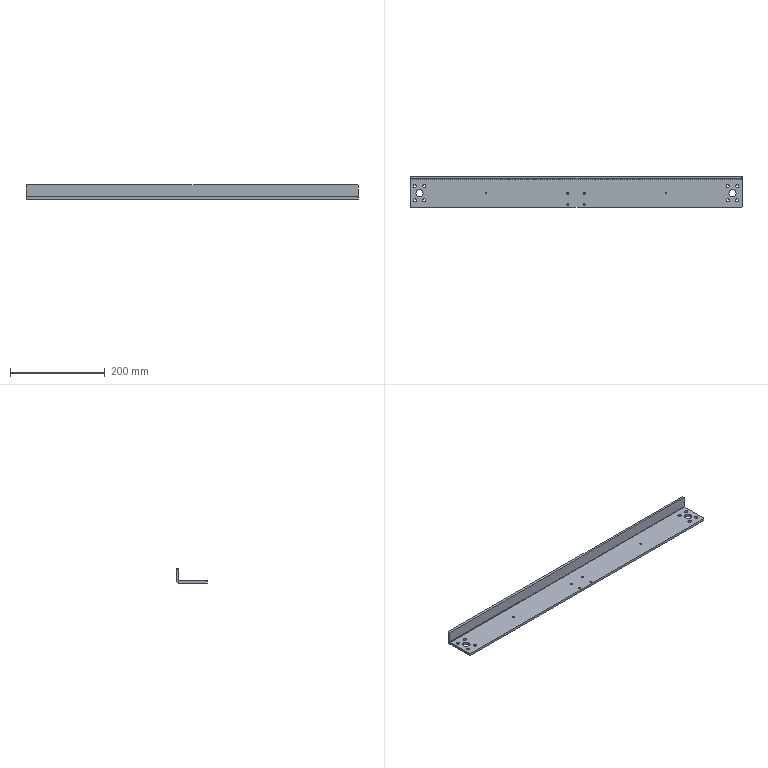Part | SolidWorks | features BaseBody 1 | 1 solid | 46 faces | box 702 x 65 x 30 mm | volume 307486 mm3 | cylinder 34 | plane 12 | commonest cylinder face diameters 6.6 x16 4.2 x8 3.3 x4 15 x4 1.473 x1 11.473 x1
STEP:
#1=CARTESIAN_POINT('',(-344.3,12.5,-5.));
#2=VERTEX_POINT('',#1);
#3=CARTESIAN_POINT('',(-337.7,12.5,-5.));
#4=VERTEX_POINT('',#3);
#5=CARTESIAN_POINT('',(-341.,12.5,-5.));
#6=DIRECTION('',(0.,0.,1.));
#7=DIRECTION('',(1.,0.,0.));
#8=AXIS2_PLACEMENT_3D('',#5,#6,#7);
#9=CIRCLE('',#8,3.3);
#10=EDGE_CURVE('',#2,#4,#9,.T.);
#11=ORIENTED_EDGE('',*,*,#10,.F.);
#12=CARTESIAN_POINT('',(-344.3,12.5,0.));
#13=VERTEX_POINT('',#12);
#14=CARTESIAN_POINT('',(-344.3,12.5,0.));
#15=DIRECTION('',(0.,0.,1.));
#16=VECTOR('',#15,1000.);
#17=LINE('',#14,#16);
#18=EDGE_CURVE('',#2,#13,#17,.T.);
#19=ORIENTED_EDGE('',*,*,#18,.T.);
#20=CARTESIAN_POINT('',(-337.7,12.5,0.));
#21=VERTEX_POINT('',#20);
#22=CARTESIAN_POINT('',(-341.,12.5,0.));
#23=DIRECTION('',(0.,0.,1.));
#24=DIRECTION('',(1.,0.,0.));
#25=AXIS2_PLACEMENT_3D('',#22,#23,#24);
#26=CIRCLE('',#25,3.3);
#27=EDGE_CURVE('',#13,#21,#26,.T.);
#28=ORIENTED_EDGE('',*,*,#27,.T.);
#29=CARTESIAN_POINT('',(-337.7,12.5,0.));
#30=DIRECTION('',(0.,0.,1.));
#31=VECTOR('',#30,1000.);
#32=LINE('',#29,#31);
#33=EDGE_CURVE('',#4,#21,#32,.T.);
#34=ORIENTED_EDGE('',*,*,#33,.F.);
#35=EDGE_LOOP('',(#11,#19,#28,#34));
#36=FACE_OUTER_BOUND('',#35,.T.);
#37=CARTESIAN_POINT('',(-341.,12.5,0.));
#38=DIRECTION('',(0.,0.,1.));
#39=DIRECTION('',(1.,0.,0.));
#40=AXIS2_PLACEMENT_3D('',#37,#38,#39);
#41=CYLINDRICAL_SURFACE('',#40,3.3);
#42=ADVANCED_FACE('',(#36),#41,.F.);
#43=CARTESIAN_POINT('',(-324.3,12.5,-5.));
#44=VERTEX_POINT('',#43);
#45=CARTESIAN_POINT('',(-317.7,12.5,-5.));
#46=VERTEX_POINT('',#45);
#47=CARTESIAN_POINT('',(-321.,12.5,-5.));
#48=DIRECTION('',(0.,0.,1.));
#49=DIRECTION('',(1.,0.,0.));
#50=AXIS2_PLACEMENT_3D('',#47,#48,#49);
#51=CIRCLE('',#50,3.3);
#52=EDGE_CURVE('',#44,#46,#51,.T.);
#53=ORIENTED_EDGE('',*,*,#52,.F.);
#54=CARTESIAN_POINT('',(-324.3,12.5,0.));
#55=VERTEX_POINT('',#54);
#56=CARTESIAN_POINT('',(-324.3,12.5,0.));
#57=DIRECTION('',(0.,0.,1.));
#58=VECTOR('',#57,1000.);
#59=LINE('',#56,#58);
#60=EDGE_CURVE('',#44,#55,#59,.T.);
#61=ORIENTED_EDGE('',*,*,#60,.T.);
#62=CARTESIAN_POINT('',(-317.7,12.5,0.));
#63=VERTEX_POINT('',#62);
#64=CARTESIAN_POINT('',(-321.,12.5,0.));
#65=DIRECTION('',(0.,0.,1.));
#66=DIRECTION('',(1.,0.,0.));
#67=AXIS2_PLACEMENT_3D('',#64,#65,#66);
#68=CIRCLE('',#67,3.3);
#69=EDGE_CURVE('',#55,#63,#68,.T.);
#70=ORIENTED_EDGE('',*,*,#69,.T.);
#71=CARTESIAN_POINT('',(-317.7,12.5,0.));
#72=DIRECTION('',(0.,0.,1.));
#73=VECTOR('',#72,1000.);
#74=LINE('',#71,#73);
#75=EDGE_CURVE('',#46,#63,#74,.T.);
#76=ORIENTED_EDGE('',*,*,#75,.F.);
#77=EDGE_LOOP('',(#53,#61,#70,#76));
#78=FACE_OUTER_BOUND('',#77,.T.);
#79=CARTESIAN_POINT('',(-321.,12.5,0.));
#80=DIRECTION('',(0.,0.,1.));
#81=DIRECTION('',(1.,0.,0.));
#82=AXIS2_PLACEMENT_3D('',#79,#80,#81);
#83=CYLINDRICAL_SURFACE('',#82,3.3);
#84=ADVANCED_FACE('',(#78),#83,.F.);
#85=CARTESIAN_POINT('',(-324.3,-17.5,-5.));
#86=VERTEX_POINT('',#85);
#87=CARTESIAN_POINT('',(-317.7,-17.5,-5.));
#88=VERTEX_POINT('',#87);
#89=CARTESIAN_POINT('',(-321.,-17.5,-5.));
#90=DIRECTION('',(0.,0.,1.));
#91=DIRECTION('',(1.,0.,0.));
#92=AXIS2_PLACEMENT_3D('',#89,#90,#91);
#93=CIRCLE('',#92,3.3);
#94=EDGE_CURVE('',#86,#88,#93,.T.);
#95=ORIENTED_EDGE('',*,*,#94,.F.);
#96=CARTESIAN_POINT('',(-324.3,-17.5,0.));
#97=VERTEX_POINT('',#96);
#98=CARTESIAN_POINT('',(-324.3,-17.5,0.));
#99=DIRECTION('',(0.,0.,1.));
#100=VECTOR('',#99,1000.);
#101=LINE('',#98,#100);
#102=EDGE_CURVE('',#86,#97,#101,.T.);
#103=ORIENTED_EDGE('',*,*,#102,.T.);
#104=CARTESIAN_POINT('',(-317.7,-17.5,0.));
#105=VERTEX_POINT('',#104);
#106=CARTESIAN_POINT('',(-321.,-17.5,0.));
#107=DIRECTION('',(0.,0.,1.));
#108=DIRECTION('',(1.,0.,0.));
#109=AXIS2_PLACEMENT_3D('',#106,#107,#108);
#110=CIRCLE('',#109,3.3);
#111=EDGE_CURVE('',#97,#105,#110,.T.);
#112=ORIENTED_EDGE('',*,*,#111,.T.);
#113=CARTESIAN_POINT('',(-317.7,-17.5,0.));
#114=DIRECTION('',(0.,0.,1.));
#115=VECTOR('',#114,1000.);
#116=LINE('',#113,#115);
#117=EDGE_CURVE('',#88,#105,#116,.T.);
#118=ORIENTED_EDGE('',*,*,#117,.F.);
#119=EDGE_LOOP('',(#95,#103,#112,#118));
#120=FACE_OUTER_BOUND('',#119,.T.);
#121=CARTESIAN_POINT('',(-321.,-17.5,0.));
#122=DIRECTION('',(0.,0.,1.));
#123=DIRECTION('',(1.,0.,0.));
#124=AXIS2_PLACEMENT_3D('',#121,#122,#123);
#125=CYLINDRICAL_SURFACE('',#124,3.3);
#126=ADVANCED_FACE('',(#120),#125,.F.);
#127=CARTESIAN_POINT('',(-344.3,-17.5,-5.));
#128=VERTEX_POINT('',#127);
#129=CARTESIAN_POINT('',(-337.7,-17.5,-5.));
#130=VERTEX_POINT('',#129);
#131=CARTESIAN_POINT('',(-341.,-17.5,-5.));
#132=DIRECTION('',(0.,0.,1.));
#133=DIRECTION('',(1.,0.,0.));
#134=AXIS2_PLACEMENT_3D('',#131,#132,#133);
#135=CIRCLE('',#134,3.3);
#136=EDGE_CURVE('',#128,#130,#135,.T.);
#137=ORIENTED_EDGE('',*,*,#136,.F.);
#138=CARTESIAN_POINT('',(-344.3,-17.5,0.));
#139=VERTEX_POINT('',#138);
#140=CARTESIAN_POINT('',(-344.3,-17.5,0.));
#141=DIRECTION('',(0.,0.,1.));
#142=VECTOR('',#141,1000.);
#143=LINE('',#140,#142);
#144=EDGE_CURVE('',#128,#139,#143,.T.);
#145=ORIENTED_EDGE('',*,*,#144,.T.);
#146=CARTESIAN_POINT('',(-337.7,-17.5,0.));
#147=VERTEX_POINT('',#146);
#148=CARTESIAN_POINT('',(-341.,-17.5,0.));
#149=DIRECTION('',(0.,0.,1.));
#150=DIRECTION('',(1.,0.,0.));
#151=AXIS2_PLACEMENT_3D('',#148,#149,#150);
#152=CIRCLE('',#151,3.3);
#153=EDGE_CURVE('',#139,#147,#152,.T.);
#154=ORIENTED_EDGE('',*,*,#153,.T.);
#155=CARTESIAN_POINT('',(-337.7,-17.5,0.));
#156=DIRECTION('',(0.,0.,1.));
#157=VECTOR('',#156,1000.);
#158=LINE('',#155,#157);
#159=EDGE_CURVE('',#130,#147,#158,.T.);
#160=ORIENTED_EDGE('',*,*,#159,.F.);
#161=EDGE_LOOP('',(#137,#145,#154,#160));
#162=FACE_OUTER_BOUND('',#161,.T.);
#163=CARTESIAN_POINT('',(-341.,-17.5,0.));
#164=DIRECTION('',(0.,0.,1.));
#165=DIRECTION('',(1.,0.,0.));
#166=AXIS2_PLACEMENT_3D('',#163,#164,#165);
#167=CYLINDRICAL_SURFACE('',#166,3.3);
#168=ADVANCED_FACE('',(#162),#167,.F.);
#169=CARTESIAN_POINT('',(317.7,12.5,-5.));
#170=VERTEX_POINT('',#169);
#171=CARTESIAN_POINT('',(324.3,12.5,-5.));
#172=VERTEX_POINT('',#171);
#173=CARTESIAN_POINT('',(321.,12.5,-5.));
#174=DIRECTION('',(0.,0.,1.));
#175=DIRECTION('',(1.,0.,0.));
#176=AXIS2_PLACEMENT_3D('',#173,#174,#175);
#177=CIRCLE('',#176,3.3);
#178=EDGE_CURVE('',#170,#172,#177,.T.);
#179=ORIENTED_EDGE('',*,*,#178,.F.);
#180=CARTESIAN_POINT('',(317.7,12.5,0.));
#181=VERTEX_POINT('',#180);
#182=CARTESIAN_POINT('',(317.7,12.5,0.));
#183=DIRECTION('',(0.,0.,1.));
#184=VECTOR('',#183,1000.);
#185=LINE('',#182,#184);
#186=EDGE_CURVE('',#170,#181,#185,.T.);
#187=ORIENTED_EDGE('',*,*,#186,.T.);
#188=CARTESIAN_POINT('',(324.3,12.5,0.));
#189=VERTEX_POINT('',#188);
#190=CARTESIAN_POINT('',(321.,12.5,0.));
#191=DIRECTION('',(0.,0.,1.));
#192=DIRECTION('',(1.,0.,0.));
#193=AXIS2_PLACEMENT_3D('',#190,#191,#192);
#194=CIRCLE('',#193,3.3);
#195=EDGE_CURVE('',#181,#189,#194,.T.);
#196=ORIENTED_EDGE('',*,*,#195,.T.);
#197=CARTESIAN_POINT('',(324.3,12.5,0.));
#198=DIRECTION('',(0.,0.,1.));
#199=VECTOR('',#198,1000.);
#200=LINE('',#197,#199);
#201=EDGE_CURVE('',#172,#189,#200,.T.);
#202=ORIENTED_EDGE('',*,*,#201,.F.);
#203=EDGE_LOOP('',(#179,#187,#196,#202));
#204=FACE_OUTER_BOUND('',#203,.T.);
#205=CARTESIAN_POINT('',(321.,12.5,0.));
#206=DIRECTION('',(0.,0.,1.));
#207=DIRECTION('',(1.,0.,0.));
#208=AXIS2_PLACEMENT_3D('',#205,#206,#207);
#209=CYLINDRICAL_SURFACE('',#208,3.3);
#210=ADVANCED_FACE('',(#204),#209,.F.);
#211=CARTESIAN_POINT('',(337.7,12.5,-5.));
#212=VERTEX_POINT('',#211);
#213=CARTESIAN_POINT('',(344.3,12.5,-5.));
#214=VERTEX_POINT('',#213);
#215=CARTESIAN_POINT('',(341.,12.5,-5.));
#216=DIRECTION('',(0.,0.,1.));
#217=DIRECTION('',(1.,0.,0.));
#218=AXIS2_PLACEMENT_3D('',#215,#216,#217);
#219=CIRCLE('',#218,3.3);
#220=EDGE_CURVE('',#212,#214,#219,.T.);
#221=ORIENTED_EDGE('',*,*,#220,.F.);
#222=CARTESIAN_POINT('',(337.7,12.5,0.));
#223=VERTEX_POINT('',#222);
#224=CARTESIAN_POINT('',(337.7,12.5,0.));
#225=DIRECTION('',(0.,0.,1.));
#226=VECTOR('',#225,1000.);
#227=LINE('',#224,#226);
#228=EDGE_CURVE('',#212,#223,#227,.T.);
#229=ORIENTED_EDGE('',*,*,#228,.T.);
#230=CARTESIAN_POINT('',(344.3,12.5,0.));
#231=VERTEX_POINT('',#230);
#232=CARTESIAN_POINT('',(341.,12.5,0.));
#233=DIRECTION('',(0.,0.,1.));
#234=DIRECTION('',(1.,0.,0.));
#235=AXIS2_PLACEMENT_3D('',#232,#233,#234);
#236=CIRCLE('',#235,3.3);
#237=EDGE_CURVE('',#223,#231,#236,.T.);
#238=ORIENTED_EDGE('',*,*,#237,.T.);
#239=CARTESIAN_POINT('',(344.3,12.5,0.));
#240=DIRECTION('',(0.,0.,1.));
#241=VECTOR('',#240,1000.);
#242=LINE('',#239,#241);
#243=EDGE_CURVE('',#214,#231,#242,.T.);
#244=ORIENTED_EDGE('',*,*,#243,.F.);
#245=EDGE_LOOP('',(#221,#229,#238,#244));
#246=FACE_OUTER_BOUND('',#245,.T.);
#247=CARTESIAN_POINT('',(341.,12.5,0.));
#248=DIRECTION('',(0.,0.,1.));
#249=DIRECTION('',(1.,0.,0.));
#250=AXIS2_PLACEMENT_3D('',#247,#248,#249);
#251=CYLINDRICAL_SURFACE('',#250,3.3);
#252=ADVANCED_FACE('',(#246),#251,.F.);
#253=CARTESIAN_POINT('',(337.7,-17.5,-5.));
#254=VERTEX_POINT('',#253);
#255=CARTESIAN_POINT('',(344.3,-17.5,-5.));
#256=VERTEX_POINT('',#255);
#257=CARTESIAN_POINT('',(341.,-17.5,-5.));
#258=DIRECTION('',(0.,0.,1.));
#259=DIRECTION('',(1.,0.,0.));
#260=AXIS2_PLACEMENT_3D('',#257,#258,#259);
#261=CIRCLE('',#260,3.3);
#262=EDGE_CURVE('',#254,#256,#261,.T.);
#263=ORIENTED_EDGE('',*,*,#262,.F.);
#264=CARTESIAN_POINT('',(337.7,-17.5,0.));
#265=VERTEX_POINT('',#264);
#266=CARTESIAN_POINT('',(337.7,-17.5,0.));
#267=DIRECTION('',(0.,0.,1.));
#268=VECTOR('',#267,1000.);
#269=LINE('',#266,#268);
#270=EDGE_CURVE('',#254,#265,#269,.T.);
#271=ORIENTED_EDGE('',*,*,#270,.T.);
#272=CARTESIAN_POINT('',(344.3,-17.5,0.));
#273=VERTEX_POINT('',#272);
#274=CARTESIAN_POINT('',(341.,-17.5,0.));
#275=DIRECTION('',(0.,0.,1.));
#276=DIRECTION('',(1.,0.,0.));
#277=AXIS2_PLACEMENT_3D('',#274,#275,#276);
#278=CIRCLE('',#277,3.3);
#279=EDGE_CURVE('',#265,#273,#278,.T.);
#280=ORIENTED_EDGE('',*,*,#279,.T.);
#281=CARTESIAN_POINT('',(344.3,-17.5,0.));
#282=DIRECTION('',(0.,0.,1.));
#283=VECTOR('',#282,1000.);
#284=LINE('',#281,#283);
#285=EDGE_CURVE('',#256,#273,#284,.T.);
#286=ORIENTED_EDGE('',*,*,#285,.F.);
#287=EDGE_LOOP('',(#263,#271,#280,#286));
#288=FACE_OUTER_BOUND('',#287,.T.);
#289=CARTESIAN_POINT('',(341.,-17.5,0.));
#290=DIRECTION('',(0.,0.,1.));
#291=DIRECTION('',(1.,0.,0.));
#292=AXIS2_PLACEMENT_3D('',#289,#290,#291);
#293=CYLINDRICAL_SURFACE('',#292,3.3);
#294=ADVANCED_FACE('',(#288),#293,.F.);
#295=CARTESIAN_POINT('',(317.7,-17.5,-5.));
#296=VERTEX_POINT('',#295);
#297=CARTESIAN_POINT('',(324.3,-17.5,-5.));
#298=VERTEX_POINT('',#297);
#299=CARTESIAN_POINT('',(321.,-17.5,-5.));
#300=DIRECTION('',(0.,0.,1.));
#301=DIRECTION('',(1.,0.,0.));
#302=AXIS2_PLACEMENT_3D('',#299,#300,#301);
#303=CIRCLE('',#302,3.3);
#304=EDGE_CURVE('',#296,#298,#303,.T.);
#305=ORIENTED_EDGE('',*,*,#304,.F.);
#306=CARTESIAN_POINT('',(317.7,-17.5,0.));
#307=VERTEX_POINT('',#306);
#308=CARTESIAN_POINT('',(317.7,-17.5,0.));
#309=DIRECTION('',(0.,0.,1.));
#310=VECTOR('',#309,1000.);
#311=LINE('',#308,#310);
#312=EDGE_CURVE('',#296,#307,#311,.T.);
#313=ORIENTED_EDGE('',*,*,#312,.T.);
#314=CARTESIAN_POINT('',(324.3,-17.5,0.));
#315=VERTEX_POINT('',#314);
#316=CARTESIAN_POINT('',(321.,-17.5,0.));
#317=DIRECTION('',(0.,0.,1.));
#318=DIRECTION('',(1.,0.,0.));
#319=AXIS2_PLACEMENT_3D('',#316,#317,#318);
#320=CIRCLE('',#319,3.3);
#321=EDGE_CURVE('',#307,#315,#320,.T.);
#322=ORIENTED_EDGE('',*,*,#321,.T.);
#323=CARTESIAN_POINT('',(324.3,-17.5,0.));
#324=DIRECTION('',(0.,0.,1.));
#325=VECTOR('',#324,1000.);
#326=LINE('',#323,#325);
#327=EDGE_CURVE('',#298,#315,#326,.T.);
#328=ORIENTED_EDGE('',*,*,#327,.F.);
#329=EDGE_LOOP('',(#305,#313,#322,#328));
#330=FACE_OUTER_BOUND('',#329,.T.);
#331=CARTESIAN_POINT('',(321.,-17.5,0.));
#332=DIRECTION('',(0.,0.,1.));
#333=DIRECTION('',(1.,0.,0.));
#334=AXIS2_PLACEMENT_3D('',#331,#332,#333);
#335=CYLINDRICAL_SURFACE('',#334,3.3);
#336=ADVANCED_FACE('',(#330),#335,.F.);
#337=CARTESIAN_POINT('',(-19.1,-2.5,-5.));
#338=VERTEX_POINT('',#337);
#339=CARTESIAN_POINT('',(-14.9,-2.5,-5.));
#340=VERTEX_POINT('',#339);
#341=CARTESIAN_POINT('',(-17.,-2.5,-5.));
#342=DIRECTION('',(0.,0.,1.));
#343=DIRECTION('',(1.,0.,0.));
#344=AXIS2_PLACEMENT_3D('',#341,#342,#343);
#345=CIRCLE('',#344,2.1);
#346=EDGE_CURVE('',#338,#340,#345,.T.);
#347=ORIENTED_EDGE('',*,*,#346,.F.);
#348=CARTESIAN_POINT('',(-19.1,-2.5,0.));
#349=VERTEX_POINT('',#348);
#350=CARTESIAN_POINT('',(-19.1,-2.5,0.));
#351=DIRECTION('',(0.,0.,1.));
#352=VECTOR('',#351,1000.);
#353=LINE('',#350,#352);
#354=EDGE_CURVE('',#338,#349,#353,.T.);
#355=ORIENTED_EDGE('',*,*,#354,.T.);
#356=CARTESIAN_POINT('',(-14.9,-2.5,0.));
#357=VERTEX_POINT('',#356);
#358=CARTESIAN_POINT('',(-17.,-2.5,0.));
#359=DIRECTION('',(0.,0.,1.));
#360=DIRECTION('',(1.,0.,0.));
#361=AXIS2_PLACEMENT_3D('',#358,#359,#360);
#362=CIRCLE('',#361,2.1);
#363=EDGE_CURVE('',#349,#357,#362,.T.);
#364=ORIENTED_EDGE('',*,*,#363,.T.);
#365=CARTESIAN_POINT('',(-14.9,-2.5,0.));
#366=DIRECTION('',(0.,0.,1.));
#367=VECTOR('',#366,1000.);
#368=LINE('',#365,#367);
#369=EDGE_CURVE('',#340,#357,#368,.T.);
#370=ORIENTED_EDGE('',*,*,#369,.F.);
#371=EDGE_LOOP('',(#347,#355,#364,#370));
#372=FACE_OUTER_BOUND('',#371,.T.);
#373=CARTESIAN_POINT('',(-17.,-2.5,0.));
#374=DIRECTION('',(0.,0.,1.));
#375=DIRECTION('',(1.,0.,0.));
#376=AXIS2_PLACEMENT_3D('',#373,#374,#375);
#377=CYLINDRICAL_SURFACE('',#376,2.1);
#378=ADVANCED_FACE('',(#372),#377,.F.);
#379=CARTESIAN_POINT('',(-19.1,-26.5,-5.));
#380=VERTEX_POINT('',#379);
#381=CARTESIAN_POINT('',(-14.9,-26.5,-5.));
#382=VERTEX_POINT('',#381);
#383=CARTESIAN_POINT('',(-17.,-26.5,-5.));
#384=DIRECTION('',(0.,0.,1.));
#385=DIRECTION('',(1.,0.,0.));
#386=AXIS2_PLACEMENT_3D('',#383,#384,#385);
#387=CIRCLE('',#386,2.1);
#388=EDGE_CURVE('',#380,#382,#387,.T.);
#389=ORIENTED_EDGE('',*,*,#388,.F.);
#390=CARTESIAN_POINT('',(-19.1,-26.5,0.));
#391=VERTEX_POINT('',#390);
#392=CARTESIAN_POINT('',(-19.1,-26.5,0.));
#393=DIRECTION('',(0.,0.,1.));
#394=VECTOR('',#393,1000.);
#395=LINE('',#392,#394);
#396=EDGE_CURVE('',#380,#391,#395,.T.);
#397=ORIENTED_EDGE('',*,*,#396,.T.);
#398=CARTESIAN_POINT('',(-14.9,-26.5,0.));
#399=VERTEX_POINT('',#398);
#400=CARTESIAN_POINT('',(-17.,-26.5,0.));
#401=DIRECTION('',(0.,0.,1.));
#402=DIRECTION('',(1.,0.,0.));
#403=AXIS2_PLACEMENT_3D('',#400,#401,#402);
#404=CIRCLE('',#403,2.1);
#405=EDGE_CURVE('',#391,#399,#404,.T.);
#406=ORIENTED_EDGE('',*,*,#405,.T.);
#407=CARTESIAN_POINT('',(-14.9,-26.5,0.));
#408=DIRECTION('',(0.,0.,1.));
#409=VECTOR('',#408,1000.);
#410=LINE('',#407,#409);
#411=EDGE_CURVE('',#382,#399,#410,.T.);
#412=ORIENTED_EDGE('',*,*,#411,.F.);
#413=EDGE_LOOP('',(#389,#397,#406,#412));
#414=FACE_OUTER_BOUND('',#413,.T.);
#415=CARTESIAN_POINT('',(-17.,-26.5,0.));
#416=DIRECTION('',(0.,0.,1.));
#417=DIRECTION('',(1.,0.,0.));
#418=AXIS2_PLACEMENT_3D('',#415,#416,#417);
#419=CYLINDRICAL_SURFACE('',#418,2.1);
#420=ADVANCED_FACE('',(#414),#419,.F.);
#421=CARTESIAN_POINT('',(14.9,-26.5,-5.));
#422=VERTEX_POINT('',#421);
#423=CARTESIAN_POINT('',(19.1,-26.5,-5.));
#424=VERTEX_POINT('',#423);
#425=CARTESIAN_POINT('',(17.,-26.5,-5.));
#426=DIRECTION('',(0.,0.,1.));
#427=DIRECTION('',(1.,0.,0.));
#428=AXIS2_PLACEMENT_3D('',#425,#426,#427);
#429=CIRCLE('',#428,2.1);
#430=EDGE_CURVE('',#422,#424,#429,.T.);
#431=ORIENTED_EDGE('',*,*,#430,.F.);
#432=CARTESIAN_POINT('',(14.9,-26.5,0.));
#433=VERTEX_POINT('',#432);
#434=CARTESIAN_POINT('',(14.9,-26.5,0.));
#435=DIRECTION('',(0.,0.,1.));
#436=VECTOR('',#435,1000.);
#437=LINE('',#434,#436);
#438=EDGE_CURVE('',#422,#433,#437,.T.);
#439=ORIENTED_EDGE('',*,*,#438,.T.);
#440=CARTESIAN_POINT('',(19.1,-26.5,0.));
#441=VERTEX_POINT('',#440);
#442=CARTESIAN_POINT('',(17.,-26.5,0.));
#443=DIRECTION('',(0.,0.,1.));
#444=DIRECTION('',(1.,0.,0.));
#445=AXIS2_PLACEMENT_3D('',#442,#443,#444);
#446=CIRCLE('',#445,2.1);
#447=EDGE_CURVE('',#433,#441,#446,.T.);
#448=ORIENTED_EDGE('',*,*,#447,.T.);
#449=CARTESIAN_POINT('',(19.1,-26.5,0.));
#450=DIRECTION('',(0.,0.,1.));
#451=VECTOR('',#450,1000.);
#452=LINE('',#449,#451);
#453=EDGE_CURVE('',#424,#441,#452,.T.);
#454=ORIENTED_EDGE('',*,*,#453,.F.);
#455=EDGE_LOOP('',(#431,#439,#448,#454));
#456=FACE_OUTER_BOUND('',#455,.T.);
#457=CARTESIAN_POINT('',(17.,-26.5,0.));
#458=DIRECTION('',(0.,0.,1.));
#459=DIRECTION('',(1.,0.,0.));
#460=AXIS2_PLACEMENT_3D('',#457,#458,#459);
#461=CYLINDRICAL_SURFACE('',#460,2.1);
#462=ADVANCED_FACE('',(#456),#461,.F.);
#463=CARTESIAN_POINT('',(14.9,-2.5,-5.));
#464=VERTEX_POINT('',#463);
#465=CARTESIAN_POINT('',(19.1,-2.5,-5.));
#466=VERTEX_POINT('',#465);
#467=CARTESIAN_POINT('',(17.,-2.5,-5.));
#468=DIRECTION('',(0.,0.,1.));
#469=DIRECTION('',(1.,0.,0.));
#470=AXIS2_PLACEMENT_3D('',#467,#468,#469);
#471=CIRCLE('',#470,2.1);
#472=EDGE_CURVE('',#464,#466,#471,.T.);
#473=ORIENTED_EDGE('',*,*,#472,.F.);
#474=CARTESIAN_POINT('',(14.9,-2.5,0.));
#475=VERTEX_POINT('',#474);
#476=CARTESIAN_POINT('',(14.9,-2.5,0.));
#477=DIRECTION('',(0.,0.,1.));
#478=VECTOR('',#477,1000.);
#479=LINE('',#476,#478);
#480=EDGE_CURVE('',#464,#475,#479,.T.);
#481=ORIENTED_EDGE('',*,*,#480,.T.);
#482=CARTESIAN_POINT('',(19.1,-2.5,0.));
#483=VERTEX_POINT('',#482);
#484=CARTESIAN_POINT('',(17.,-2.5,0.));
#485=DIRECTION('',(0.,0.,1.));
#486=DIRECTION('',(1.,0.,0.));
#487=AXIS2_PLACEMENT_3D('',#484,#485,#486);
#488=CIRCLE('',#487,2.1);
#489=EDGE_CURVE('',#475,#483,#488,.T.);
#490=ORIENTED_EDGE('',*,*,#489,.T.);
#491=CARTESIAN_POINT('',(19.1,-2.5,0.));
#492=DIRECTION('',(0.,0.,1.));
#493=VECTOR('',#492,1000.);
#494=LINE('',#491,#493);
#495=EDGE_CURVE('',#466,#483,#494,.T.);
#496=ORIENTED_EDGE('',*,*,#495,.F.);
#497=EDGE_LOOP('',(#473,#481,#490,#496));
#498=FACE_OUTER_BOUND('',#497,.T.);
#499=CARTESIAN_POINT('',(17.,-2.5,0.));
#500=DIRECTION('',(0.,0.,1.));
#501=DIRECTION('',(1.,0.,0.));
#502=AXIS2_PLACEMENT_3D('',#499,#500,#501);
#503=CYLINDRICAL_SURFACE('',#502,2.1);
#504=ADVANCED_FACE('',(#498),#503,.F.);
#505=CARTESIAN_POINT('',(-338.5,-2.5,0.));
#506=VERTEX_POINT('',#505);
#507=CARTESIAN_POINT('',(-323.5,-2.5,0.));
#508=VERTEX_POINT('',#507);
#509=CARTESIAN_POINT('',(-331.,-2.5,0.));
#510=DIRECTION('',(0.,0.,1.));
#511=DIRECTION('',(-1.,0.,0.));
#512=AXIS2_PLACEMENT_3D('',#509,#510,#511);
#513=CIRCLE('',#512,7.5);
#514=EDGE_CURVE('',#506,#508,#513,.T.);
#515=ORIENTED_EDGE('',*,*,#514,.T.);
#516=CARTESIAN_POINT('',(-323.5,-2.5,-5.));
#517=VERTEX_POINT('',#516);
#518=CARTESIAN_POINT('',(-323.5,-2.5,5.));
#519=DIRECTION('',(0.,0.,-1.));
#520=VECTOR('',#519,1000.);
#521=LINE('',#518,#520);
#522=EDGE_CURVE('',#508,#517,#521,.T.);
#523=ORIENTED_EDGE('',*,*,#522,.T.);
#524=CARTESIAN_POINT('',(-338.5,-2.5,-5.));
#525=VERTEX_POINT('',#524);
#526=CARTESIAN_POINT('',(-331.,-2.5,-5.));
#527=DIRECTION('',(0.,0.,1.));
#528=DIRECTION('',(-1.,0.,0.));
#529=AXIS2_PLACEMENT_3D('',#526,#527,#528);
#530=CIRCLE('',#529,7.5);
#531=EDGE_CURVE('',#525,#517,#530,.T.);
#532=ORIENTED_EDGE('',*,*,#531,.F.);
#533=CARTESIAN_POINT('',(-338.5,-2.5,5.));
#534=DIRECTION('',(0.,0.,-1.));
#535=VECTOR('',#534,1000.);
#536=LINE('',#533,#535);
#537=EDGE_CURVE('',#506,#525,#536,.T.);
#538=ORIENTED_EDGE('',*,*,#537,.F.);
#539=EDGE_LOOP('',(#515,#523,#532,#538));
#540=FACE_OUTER_BOUND('',#539,.T.);
#541=CARTESIAN_POINT('',(-331.,-2.5,5.));
#542=DIRECTION('',(0.,0.,-1.));
#543=DIRECTION('',(-1.,0.,0.));
#544=AXIS2_PLACEMENT_3D('',#541,#542,#543);
#545=CYLINDRICAL_SURFACE('',#544,7.5);
#546=ADVANCED_FACE('',(#540),#545,.F.);
#547=CARTESIAN_POINT('',(323.5,-2.5,0.));
#548=VERTEX_POINT('',#547);
#549=CARTESIAN_POINT('',(338.5,-2.5,0.));
#550=VERTEX_POINT('',#549);
#551=CARTESIAN_POINT('',(331.,-2.5,0.));
#552=DIRECTION('',(0.,0.,1.));
#553=DIRECTION('',(-1.,0.,0.));
#554=AXIS2_PLACEMENT_3D('',#551,#552,#553);
#555=CIRCLE('',#554,7.5);
#556=EDGE_CURVE('',#548,#550,#555,.T.);
#557=ORIENTED_EDGE('',*,*,#556,.T.);
#558=CARTESIAN_POINT('',(338.5,-2.5,-5.));
#559=VERTEX_POINT('',#558);
#560=CARTESIAN_POINT('',(338.5,-2.5,5.));
#561=DIRECTION('',(0.,0.,-1.));
#562=VECTOR('',#561,1000.);
#563=LINE('',#560,#562);
#564=EDGE_CURVE('',#550,#559,#563,.T.);
#565=ORIENTED_EDGE('',*,*,#564,.T.);
#566=CARTESIAN_POINT('',(323.5,-2.5,-5.));
#567=VERTEX_POINT('',#566);
#568=CARTESIAN_POINT('',(331.,-2.5,-5.));
#569=DIRECTION('',(0.,0.,1.));
#570=DIRECTION('',(-1.,0.,0.));
#571=AXIS2_PLACEMENT_3D('',#568,#569,#570);
#572=CIRCLE('',#571,7.5);
#573=EDGE_CURVE('',#567,#559,#572,.T.);
#574=ORIENTED_EDGE('',*,*,#573,.F.);
#575=CARTESIAN_POINT('',(323.5,-2.5,5.));
#576=DIRECTION('',(0.,0.,-1.));
#577=VECTOR('',#576,1000.);
#578=LINE('',#575,#577);
#579=EDGE_CURVE('',#548,#567,#578,.T.);
#580=ORIENTED_EDGE('',*,*,#579,.F.);
#581=EDGE_LOOP('',(#557,#565,#574,#580));
#582=FACE_OUTER_BOUND('',#581,.T.);
#583=CARTESIAN_POINT('',(331.,-2.5,5.));
#584=DIRECTION('',(0.,0.,-1.));
#585=DIRECTION('',(-1.,0.,0.));
#586=AXIS2_PLACEMENT_3D('',#583,#584,#585);
#587=CYLINDRICAL_SURFACE('',#586,7.5);
#588=ADVANCED_FACE('',(#582),#587,.F.);
#589=CARTESIAN_POINT('',(-191.65,-2.5,0.));
#590=VERTEX_POINT('',#589);
#591=CARTESIAN_POINT('',(-188.35,-2.5,0.));
#592=VERTEX_POINT('',#591);
#593=CARTESIAN_POINT('',(-190.,-2.5,0.));
#594=DIRECTION('',(0.,0.,1.));
#595=DIRECTION('',(-1.,0.,0.));
#596=AXIS2_PLACEMENT_3D('',#593,#594,#595);
#597=CIRCLE('',#596,1.65);
#598=EDGE_CURVE('',#590,#592,#597,.T.);
#599=ORIENTED_EDGE('',*,*,#598,.T.);
#600=CARTESIAN_POINT('',(-188.35,-2.5,-5.));
#601=VERTEX_POINT('',#600);
#602=CARTESIAN_POINT('',(-188.35,-2.5,-5.));
#603=DIRECTION('',(0.,0.,-1.));
#604=VECTOR('',#603,1000.);
#605=LINE('',#602,#604);
#606=EDGE_CURVE('',#592,#601,#605,.T.);
#607=ORIENTED_EDGE('',*,*,#606,.T.);
#608=CARTESIAN_POINT('',(-191.65,-2.5,-5.));
#609=VERTEX_POINT('',#608);
#610=CARTESIAN_POINT('',(-190.,-2.5,-5.));
#611=DIRECTION('',(0.,0.,1.));
#612=DIRECTION('',(-1.,0.,0.));
#613=AXIS2_PLACEMENT_3D('',#610,#611,#612);
#614=CIRCLE('',#613,1.65);
#615=EDGE_CURVE('',#609,#601,#614,.T.);
#616=ORIENTED_EDGE('',*,*,#615,.F.);
#617=CARTESIAN_POINT('',(-191.65,-2.5,-5.));
#618=DIRECTION('',(0.,0.,-1.));
#619=VECTOR('',#618,1000.);
#620=LINE('',#617,#619);
#621=EDGE_CURVE('',#590,#609,#620,.T.);
#622=ORIENTED_EDGE('',*,*,#621,.F.);
#623=EDGE_LOOP('',(#599,#607,#616,#622));
#624=FACE_OUTER_BOUND('',#623,.T.);
#625=CARTESIAN_POINT('',(-190.,-2.5,-5.));
#626=DIRECTION('',(0.,0.,-1.));
#627=DIRECTION('',(-1.,0.,0.));
#628=AXIS2_PLACEMENT_3D('',#625,#626,#627);
#629=CYLINDRICAL_SURFACE('',#628,1.65);
#630=ADVANCED_FACE('',(#624),#629,.F.);
#631=CARTESIAN_POINT('',(188.35,-2.5,0.));
#632=VERTEX_POINT('',#631);
#633=CARTESIAN_POINT('',(191.65,-2.5,0.));
#634=VERTEX_POINT('',#633);
#635=CARTESIAN_POINT('',(190.,-2.5,0.));
#636=DIRECTION('',(0.,0.,1.));
#637=DIRECTION('',(-1.,0.,0.));
#638=AXIS2_PLACEMENT_3D('',#635,#636,#637);
#639=CIRCLE('',#638,1.65);
#640=EDGE_CURVE('',#632,#634,#639,.T.);
#641=ORIENTED_EDGE('',*,*,#640,.T.);
#642=CARTESIAN_POINT('',(191.65,-2.5,-5.));
#643=VERTEX_POINT('',#642);
#644=CARTESIAN_POINT('',(191.65,-2.5,-5.));
#645=DIRECTION('',(0.,0.,-1.));
#646=VECTOR('',#645,1000.);
#647=LINE('',#644,#646);
#648=EDGE_CURVE('',#634,#643,#647,.T.);
#649=ORIENTED_EDGE('',*,*,#648,.T.);
#650=CARTESIAN_POINT('',(188.35,-2.5,-5.));
#651=VERTEX_POINT('',#650);
#652=CARTESIAN_POINT('',(190.,-2.5,-5.));
#653=DIRECTION('',(0.,0.,1.));
#654=DIRECTION('',(-1.,0.,0.));
#655=AXIS2_PLACEMENT_3D('',#652,#653,#654);
#656=CIRCLE('',#655,1.65);
#657=EDGE_CURVE('',#651,#643,#656,.T.);
#658=ORIENTED_EDGE('',*,*,#657,.F.);
#659=CARTESIAN_POINT('',(188.35,-2.5,-5.));
#660=DIRECTION('',(0.,0.,-1.));
#661=VECTOR('',#660,1000.);
#662=LINE('',#659,#661);
#663=EDGE_CURVE('',#632,#651,#662,.T.);
#664=ORIENTED_EDGE('',*,*,#663,.F.);
#665=EDGE_LOOP('',(#641,#649,#658,#664));
#666=FACE_OUTER_BOUND('',#665,.T.);
#667=CARTESIAN_POINT('',(190.,-2.5,-5.));
#668=DIRECTION('',(0.,0.,-1.));
#669=DIRECTION('',(-1.,0.,0.));
#670=AXIS2_PLACEMENT_3D('',#667,#668,#669);
#671=CYLINDRICAL_SURFACE('',#670,1.65);
#672=ADVANCED_FACE('',(#666),#671,.F.);
#673=CARTESIAN_POINT('',(-349.,-32.5,0.));
#674=VERTEX_POINT('',#673);
#675=CARTESIAN_POINT('',(-351.,-30.5,0.));
#676=VERTEX_POINT('',#675);
#677=CARTESIAN_POINT('',(-349.,-32.5,0.));
#678=DIRECTION('',(-0.7071,0.7071,0.));
#679=VECTOR('',#678,1000.);
#680=LINE('',#677,#679);
#681=EDGE_CURVE('',#674,#676,#680,.T.);
#682=ORIENTED_EDGE('',*,*,#681,.F.);
#683=CARTESIAN_POINT('',(349.,-32.5,0.));
#684=VERTEX_POINT('',#683);
#685=CARTESIAN_POINT('',(0.,-32.5,0.));
#686=DIRECTION('',(-1.,0.,0.));
#687=VECTOR('',#686,1000.);
#688=LINE('',#685,#687);
#689=EDGE_CURVE('',#684,#674,#688,.T.);
#690=ORIENTED_EDGE('',*,*,#689,.F.);
#691=CARTESIAN_POINT('',(351.,-30.5,0.));
#692=VERTEX_POINT('',#691);
#693=CARTESIAN_POINT('',(351.,-30.5,0.));
#694=DIRECTION('',(-0.7071,-0.7071,0.));
#695=VECTOR('',#694,1000.);
#696=LINE('',#693,#695);
#697=EDGE_CURVE('',#692,#684,#696,.T.);
#698=ORIENTED_EDGE('',*,*,#697,.F.);
#699=CARTESIAN_POINT('',(351.,26.763,0.));
#700=VERTEX_POINT('',#699);
#701=CARTESIAN_POINT('',(351.,0.,0.));
#702=DIRECTION('',(0.,-1.,0.));
#703=VECTOR('',#702,1000.);
#704=LINE('',#701,#703);
#705=EDGE_CURVE('',#700,#692,#704,.T.);
#706=ORIENTED_EDGE('',*,*,#705,.F.);
#707=CARTESIAN_POINT('',(-351.,26.763,0.));
#708=VERTEX_POINT('',#707);
#709=CARTESIAN_POINT('',(0.,26.763,0.));
#710=DIRECTION('',(1.,0.,0.));
#711=VECTOR('',#710,1000.);
#712=LINE('',#709,#711);
#713=EDGE_CURVE('',#708,#700,#712,.T.);
#714=ORIENTED_EDGE('',*,*,#713,.F.);
#715=CARTESIAN_POINT('',(-351.,0.,0.));
#716=DIRECTION('',(0.,1.,0.));
#717=VECTOR('',#716,1000.);
#718=LINE('',#715,#717);
#719=EDGE_CURVE('',#676,#708,#718,.T.);
#720=ORIENTED_EDGE('',*,*,#719,.F.);
#721=EDGE_LOOP('',(#682,#690,#698,#706,#714,#720));
#722=FACE_OUTER_BOUND('',#721,.T.);
#723=CARTESIAN_POINT('',(-341.,12.5,0.));
#724=DIRECTION('',(0.,0.,1.));
#725=DIRECTION('',(1.,0.,0.));
#726=AXIS2_PLACEMENT_3D('',#723,#724,#725);
#727=CIRCLE('',#726,3.3);
#728=EDGE_CURVE('',#21,#13,#727,.T.);
#729=ORIENTED_EDGE('',*,*,#728,.F.);
#730=ORIENTED_EDGE('',*,*,#27,.F.);
#731=EDGE_LOOP('',(#729,#730));
#732=FACE_BOUND('',#731,.T.);
#733=CARTESIAN_POINT('',(-321.,12.5,0.));
#734=DIRECTION('',(0.,0.,1.));
#735=DIRECTION('',(1.,0.,0.));
#736=AXIS2_PLACEMENT_3D('',#733,#734,#735);
#737=CIRCLE('',#736,3.3);
#738=EDGE_CURVE('',#63,#55,#737,.T.);
#739=ORIENTED_EDGE('',*,*,#738,.F.);
#740=ORIENTED_EDGE('',*,*,#69,.F.);
#741=EDGE_LOOP('',(#739,#740));
#742=FACE_BOUND('',#741,.T.);
#743=CARTESIAN_POINT('',(-321.,-17.5,0.));
#744=DIRECTION('',(0.,0.,1.));
#745=DIRECTION('',(1.,0.,0.));
#746=AXIS2_PLACEMENT_3D('',#743,#744,#745);
#747=CIRCLE('',#746,3.3);
#748=EDGE_CURVE('',#105,#97,#747,.T.);
#749=ORIENTED_EDGE('',*,*,#748,.F.);
#750=ORIENTED_EDGE('',*,*,#111,.F.);
#751=EDGE_LOOP('',(#749,#750));
#752=FACE_BOUND('',#751,.T.);
#753=CARTESIAN_POINT('',(-341.,-17.5,0.));
#754=DIRECTION('',(0.,0.,1.));
#755=DIRECTION('',(1.,0.,0.));
#756=AXIS2_PLACEMENT_3D('',#753,#754,#755);
#757=CIRCLE('',#756,3.3);
#758=EDGE_CURVE('',#147,#139,#757,.T.);
#759=ORIENTED_EDGE('',*,*,#758,.F.);
#760=ORIENTED_EDGE('',*,*,#153,.F.);
#761=EDGE_LOOP('',(#759,#760));
#762=FACE_BOUND('',#761,.T.);
#763=CARTESIAN_POINT('',(321.,12.5,0.));
#764=DIRECTION('',(0.,0.,1.));
#765=DIRECTION('',(1.,0.,0.));
#766=AXIS2_PLACEMENT_3D('',#763,#764,#765);
#767=CIRCLE('',#766,3.3);
#768=EDGE_CURVE('',#189,#181,#767,.T.);
#769=ORIENTED_EDGE('',*,*,#768,.F.);
#770=ORIENTED_EDGE('',*,*,#195,.F.);
#771=EDGE_LOOP('',(#769,#770));
#772=FACE_BOUND('',#771,.T.);
#773=CARTESIAN_POINT('',(341.,12.5,0.));
#774=DIRECTION('',(0.,0.,1.));
#775=DIRECTION('',(1.,0.,0.));
#776=AXIS2_PLACEMENT_3D('',#773,#774,#775);
#777=CIRCLE('',#776,3.3);
#778=EDGE_CURVE('',#231,#223,#777,.T.);
#779=ORIENTED_EDGE('',*,*,#778,.F.);
#780=ORIENTED_EDGE('',*,*,#237,.F.);
#781=EDGE_LOOP('',(#779,#780));
#782=FACE_BOUND('',#781,.T.);
#783=CARTESIAN_POINT('',(341.,-17.5,0.));
#784=DIRECTION('',(0.,0.,1.));
#785=DIRECTION('',(1.,0.,0.));
#786=AXIS2_PLACEMENT_3D('',#783,#784,#785);
#787=CIRCLE('',#786,3.3);
#788=EDGE_CURVE('',#273,#265,#787,.T.);
#789=ORIENTED_EDGE('',*,*,#788,.F.);
#790=ORIENTED_EDGE('',*,*,#279,.F.);
#791=EDGE_LOOP('',(#789,#790));
#792=FACE_BOUND('',#791,.T.);
#793=CARTESIAN_POINT('',(321.,-17.5,0.));
#794=DIRECTION('',(0.,0.,1.));
#795=DIRECTION('',(1.,0.,0.));
#796=AXIS2_PLACEMENT_3D('',#793,#794,#795);
#797=CIRCLE('',#796,3.3);
#798=EDGE_CURVE('',#315,#307,#797,.T.);
#799=ORIENTED_EDGE('',*,*,#798,.F.);
#800=ORIENTED_EDGE('',*,*,#321,.F.);
#801=EDGE_LOOP('',(#799,#800));
#802=FACE_BOUND('',#801,.T.);
#803=CARTESIAN_POINT('',(-17.,-2.5,0.));
#804=DIRECTION('',(0.,0.,1.));
#805=DIRECTION('',(1.,0.,0.));
#806=AXIS2_PLACEMENT_3D('',#803,#804,#805);
#807=CIRCLE('',#806,2.1);
#808=EDGE_CURVE('',#357,#349,#807,.T.);
#809=ORIENTED_EDGE('',*,*,#808,.F.);
#810=ORIENTED_EDGE('',*,*,#363,.F.);
#811=EDGE_LOOP('',(#809,#810));
#812=FACE_BOUND('',#811,.T.);
#813=CARTESIAN_POINT('',(-17.,-26.5,0.));
#814=DIRECTION('',(0.,0.,1.));
#815=DIRECTION('',(1.,0.,0.));
#816=AXIS2_PLACEMENT_3D('',#813,#814,#815);
#817=CIRCLE('',#816,2.1);
#818=EDGE_CURVE('',#399,#391,#817,.T.);
#819=ORIENTED_EDGE('',*,*,#818,.F.);
#820=ORIENTED_EDGE('',*,*,#405,.F.);
#821=EDGE_LOOP('',(#819,#820));
#822=FACE_BOUND('',#821,.T.);
#823=CARTESIAN_POINT('',(17.,-26.5,0.));
#824=DIRECTION('',(0.,0.,1.));
#825=DIRECTION('',(1.,0.,0.));
#826=AXIS2_PLACEMENT_3D('',#823,#824,#825);
#827=CIRCLE('',#826,2.1);
#828=EDGE_CURVE('',#441,#433,#827,.T.);
#829=ORIENTED_EDGE('',*,*,#828,.F.);
#830=ORIENTED_EDGE('',*,*,#447,.F.);
#831=EDGE_LOOP('',(#829,#830));
#832=FACE_BOUND('',#831,.T.);
#833=CARTESIAN_POINT('',(17.,-2.5,0.));
#834=DIRECTION('',(0.,0.,1.));
#835=DIRECTION('',(1.,0.,0.));
#836=AXIS2_PLACEMENT_3D('',#833,#834,#835);
#837=CIRCLE('',#836,2.1);
#838=EDGE_CURVE('',#483,#475,#837,.T.);
#839=ORIENTED_EDGE('',*,*,#838,.F.);
#840=ORIENTED_EDGE('',*,*,#489,.F.);
#841=EDGE_LOOP('',(#839,#840));
#842=FACE_BOUND('',#841,.T.);
#843=ORIENTED_EDGE('',*,*,#514,.F.);
#844=CARTESIAN_POINT('',(-331.,-2.5,0.));
#845=DIRECTION('',(0.,0.,1.));
#846=DIRECTION('',(-1.,0.,0.));
#847=AXIS2_PLACEMENT_3D('',#844,#845,#846);
#848=CIRCLE('',#847,7.5);
#849=EDGE_CURVE('',#508,#506,#848,.T.);
#850=ORIENTED_EDGE('',*,*,#849,.F.);
#851=EDGE_LOOP('',(#843,#850));
#852=FACE_BOUND('',#851,.T.);
#853=ORIENTED_EDGE('',*,*,#556,.F.);
#854=CARTESIAN_POINT('',(331.,-2.5,0.));
#855=DIRECTION('',(0.,0.,1.));
#856=DIRECTION('',(-1.,0.,0.));
#857=AXIS2_PLACEMENT_3D('',#854,#855,#856);
#858=CIRCLE('',#857,7.5);
#859=EDGE_CURVE('',#550,#548,#858,.T.);
#860=ORIENTED_EDGE('',*,*,#859,.F.);
#861=EDGE_LOOP('',(#853,#860));
#862=FACE_BOUND('',#861,.T.);
#863=ORIENTED_EDGE('',*,*,#598,.F.);
#864=CARTESIAN_POINT('',(-190.,-2.5,0.));
#865=DIRECTION('',(0.,0.,1.));
#866=DIRECTION('',(-1.,0.,0.));
#867=AXIS2_PLACEMENT_3D('',#864,#865,#866);
#868=CIRCLE('',#867,1.65);
#869=EDGE_CURVE('',#592,#590,#868,.T.);
#870=ORIENTED_EDGE('',*,*,#869,.F.);
#871=EDGE_LOOP('',(#863,#870));
#872=FACE_BOUND('',#871,.T.);
#873=ORIENTED_EDGE('',*,*,#640,.F.);
#874=CARTESIAN_POINT('',(190.,-2.5,0.));
#875=DIRECTION('',(0.,0.,1.));
#876=DIRECTION('',(-1.,0.,0.));
#877=AXIS2_PLACEMENT_3D('',#874,#875,#876);
#878=CIRCLE('',#877,1.65);
#879=EDGE_CURVE('',#634,#632,#878,.T.);
#880=ORIENTED_EDGE('',*,*,#879,.F.);
#881=EDGE_LOOP('',(#873,#880));
#882=FACE_BOUND('',#881,.T.);
#883=CARTESIAN_POINT('',(0.,0.,0.));
#884=DIRECTION('',(0.,0.,-1.));
#885=DIRECTION('',(-1.,0.,0.));
#886=AXIS2_PLACEMENT_3D('',#883,#884,#885);
#887=PLANE('',#886);
#888=ADVANCED_FACE('',(#722,#732,#742,#752,#762,#772,#782,#792,#802,#812,#822,#832,#842,#852,#862,#872,#882),#887,.F.);
#889=ORIENTED_EDGE('',*,*,#719,.T.);
#890=CARTESIAN_POINT('',(-351.,27.5,0.7366));
#891=VERTEX_POINT('',#890);
#892=CARTESIAN_POINT('',(-351.,26.763,0.7366));
#893=DIRECTION('',(1.,0.,0.));
#894=DIRECTION('',(0.,0.,1.));
#895=AXIS2_PLACEMENT_3D('',#892,#893,#894);
#896=CIRCLE('',#895,0.7366);
#897=EDGE_CURVE('',#708,#891,#896,.T.);
#898=ORIENTED_EDGE('',*,*,#897,.T.);
#899=CARTESIAN_POINT('',(-351.,27.5,23.));
#900=VERTEX_POINT('',#899);
#901=CARTESIAN_POINT('',(-351.,27.5,0.));
#902=DIRECTION('',(0.,0.,-1.));
#903=VECTOR('',#902,1000.);
#904=LINE('',#901,#903);
#905=EDGE_CURVE('',#900,#891,#904,.T.);
#906=ORIENTED_EDGE('',*,*,#905,.F.);
#907=CARTESIAN_POINT('',(-351.,32.5,23.));
#908=VERTEX_POINT('',#907);
#909=CARTESIAN_POINT('',(-351.,32.5,23.));
#910=DIRECTION('',(0.,-1.,0.));
#911=VECTOR('',#910,1000.);
#912=LINE('',#909,#911);
#913=EDGE_CURVE('',#908,#900,#912,.T.);
#914=ORIENTED_EDGE('',*,*,#913,.F.);
#915=CARTESIAN_POINT('',(-351.,32.5,0.7366));
#916=VERTEX_POINT('',#915);
#917=CARTESIAN_POINT('',(-351.,32.5,25.));
#918=DIRECTION('',(0.,0.,1.));
#919=VECTOR('',#918,1000.);
#920=LINE('',#917,#919);
#921=EDGE_CURVE('',#916,#908,#920,.T.);
#922=ORIENTED_EDGE('',*,*,#921,.F.);
#923=CARTESIAN_POINT('',(-351.,26.763,-5.));
#924=VERTEX_POINT('',#923);
#925=CARTESIAN_POINT('',(-351.,26.763,0.7366));
#926=DIRECTION('',(1.,0.,0.));
#927=DIRECTION('',(0.,0.,1.));
#928=AXIS2_PLACEMENT_3D('',#925,#926,#927);
#929=CIRCLE('',#928,5.737);
#930=EDGE_CURVE('',#924,#916,#929,.T.);
#931=ORIENTED_EDGE('',*,*,#930,.F.);
#932=CARTESIAN_POINT('',(-351.,-30.5,-5.));
#933=VERTEX_POINT('',#932);
#934=CARTESIAN_POINT('',(-351.,-32.5,-5.));
#935=DIRECTION('',(0.,-1.,0.));
#936=VECTOR('',#935,1000.);
#937=LINE('',#934,#936);
#938=EDGE_CURVE('',#924,#933,#937,.T.);
#939=ORIENTED_EDGE('',*,*,#938,.T.);
#940=CARTESIAN_POINT('',(-351.,-30.5,-5.));
#941=DIRECTION('',(0.,0.,1.));
#942=VECTOR('',#941,1000.);
#943=LINE('',#940,#942);
#944=EDGE_CURVE('',#933,#676,#943,.T.);
#945=ORIENTED_EDGE('',*,*,#944,.T.);
#946=EDGE_LOOP('',(#889,#898,#906,#914,#922,#931,#939,#945));
#947=FACE_OUTER_BOUND('',#946,.T.);
#948=CARTESIAN_POINT('',(-351.,-32.5,-5.));
#949=DIRECTION('',(-1.,0.,0.));
#950=DIRECTION('',(0.,0.,1.));
#951=AXIS2_PLACEMENT_3D('',#948,#949,#950);
#952=PLANE('',#951);
#953=ADVANCED_FACE('',(#947),#952,.T.);
#954=CARTESIAN_POINT('',(-349.,-32.5,-5.));
#955=VERTEX_POINT('',#954);
#956=CARTESIAN_POINT('',(-349.,-32.5,-5.));
#957=DIRECTION('',(0.,0.,-1.));
#958=VECTOR('',#957,1000.);
#959=LINE('',#956,#958);
#960=EDGE_CURVE('',#674,#955,#959,.T.);
#961=ORIENTED_EDGE('',*,*,#960,.F.);
#962=ORIENTED_EDGE('',*,*,#681,.T.);
#963=ORIENTED_EDGE('',*,*,#944,.F.);
#964=CARTESIAN_POINT('',(-351.,-30.5,-5.));
#965=DIRECTION('',(-0.7071,0.7071,0.));
#966=VECTOR('',#965,1000.);
#967=LINE('',#964,#966);
#968=EDGE_CURVE('',#955,#933,#967,.T.);
#969=ORIENTED_EDGE('',*,*,#968,.F.);
#970=EDGE_LOOP('',(#961,#962,#963,#969));
#971=FACE_OUTER_BOUND('',#970,.T.);
#972=CARTESIAN_POINT('',(-351.,-30.5,-5.));
#973=DIRECTION('',(0.7071,0.7071,0.));
#974=DIRECTION('',(-0.7071,0.7071,0.));
#975=AXIS2_PLACEMENT_3D('',#972,#973,#974);
#976=PLANE('',#975);
#977=ADVANCED_FACE('',(#971),#976,.F.);
#978=CARTESIAN_POINT('',(349.,-32.5,-5.));
#979=VERTEX_POINT('',#978);
#980=CARTESIAN_POINT('',(-351.,-32.5,-5.));
#981=DIRECTION('',(1.,0.,0.));
#982=VECTOR('',#981,1000.);
#983=LINE('',#980,#982);
#984=EDGE_CURVE('',#955,#979,#983,.T.);
#985=ORIENTED_EDGE('',*,*,#984,.T.);
#986=CARTESIAN_POINT('',(349.,-32.5,-5.));
#987=DIRECTION('',(0.,0.,1.));
#988=VECTOR('',#987,1000.);
#989=LINE('',#986,#988);
#990=EDGE_CURVE('',#979,#684,#989,.T.);
#991=ORIENTED_EDGE('',*,*,#990,.T.);
#992=ORIENTED_EDGE('',*,*,#689,.T.);
#993=ORIENTED_EDGE('',*,*,#960,.T.);
#994=EDGE_LOOP('',(#985,#991,#992,#993));
#995=FACE_OUTER_BOUND('',#994,.T.);
#996=CARTESIAN_POINT('',(-351.,-32.5,-5.));
#997=DIRECTION('',(0.,-1.,0.));
#998=DIRECTION('',(0.,0.,-1.));
#999=AXIS2_PLACEMENT_3D('',#996,#997,#998);
#1000=PLANE('',#999);
#1001=ADVANCED_FACE('',(#995),#1000,.T.);
#1002=CARTESIAN_POINT('',(351.,-30.5,-5.));
#1003=VERTEX_POINT('',#1002);
#1004=CARTESIAN_POINT('',(351.,-30.5,-5.));
#1005=DIRECTION('',(0.,0.,-1.));
#1006=VECTOR('',#1005,1000.);
#1007=LINE('',#1004,#1006);
#1008=EDGE_CURVE('',#692,#1003,#1007,.T.);
#1009=ORIENTED_EDGE('',*,*,#1008,.F.);
#1010=ORIENTED_EDGE('',*,*,#697,.T.);
#1011=ORIENTED_EDGE('',*,*,#990,.F.);
#1012=CARTESIAN_POINT('',(349.,-32.5,-5.));
#1013=DIRECTION('',(-0.7071,-0.7071,0.));
#1014=VECTOR('',#1013,1000.);
#1015=LINE('',#1012,#1014);
#1016=EDGE_CURVE('',#1003,#979,#1015,.T.);
#1017=ORIENTED_EDGE('',*,*,#1016,.F.);
#1018=EDGE_LOOP('',(#1009,#1010,#1011,#1017));
#1019=FACE_OUTER_BOUND('',#1018,.T.);
#1020=CARTESIAN_POINT('',(349.,-32.5,-5.));
#1021=DIRECTION('',(-0.7071,0.7071,0.));
#1022=DIRECTION('',(-0.7071,-0.7071,0.));
#1023=AXIS2_PLACEMENT_3D('',#1020,#1021,#1022);
#1024=PLANE('',#1023);
#1025=ADVANCED_FACE('',(#1019),#1024,.F.);
#1026=CARTESIAN_POINT('',(351.,26.763,-5.));
#1027=VERTEX_POINT('',#1026);
#1028=CARTESIAN_POINT('',(351.,-32.5,-5.));
#1029=DIRECTION('',(0.,1.,0.));
#1030=VECTOR('',#1029,1000.);
#1031=LINE('',#1028,#1030);
#1032=EDGE_CURVE('',#1003,#1027,#1031,.T.);
#1033=ORIENTED_EDGE('',*,*,#1032,.T.);
#1034=CARTESIAN_POINT('',(351.,32.5,0.7366));
#1035=VERTEX_POINT('',#1034);
#1036=CARTESIAN_POINT('',(351.,26.763,0.7366));
#1037=DIRECTION('',(1.,0.,0.));
#1038=DIRECTION('',(0.,0.,1.));
#1039=AXIS2_PLACEMENT_3D('',#1036,#1037,#1038);
#1040=CIRCLE('',#1039,5.737);
#1041=EDGE_CURVE('',#1027,#1035,#1040,.T.);
#1042=ORIENTED_EDGE('',*,*,#1041,.T.);
#1043=CARTESIAN_POINT('',(351.,32.5,23.));
#1044=VERTEX_POINT('',#1043);
#1045=CARTESIAN_POINT('',(351.,32.5,0.));
#1046=DIRECTION('',(0.,0.,-1.));
#1047=VECTOR('',#1046,1000.);
#1048=LINE('',#1045,#1047);
#1049=EDGE_CURVE('',#1044,#1035,#1048,.T.);
#1050=ORIENTED_EDGE('',*,*,#1049,.F.);
#1051=CARTESIAN_POINT('',(351.,27.5,23.));
#1052=VERTEX_POINT('',#1051);
#1053=CARTESIAN_POINT('',(351.,32.5,23.));
#1054=DIRECTION('',(0.,1.,0.));
#1055=VECTOR('',#1054,1000.);
#1056=LINE('',#1053,#1055);
#1057=EDGE_CURVE('',#1052,#1044,#1056,.T.);
#1058=ORIENTED_EDGE('',*,*,#1057,.F.);
#1059=CARTESIAN_POINT('',(351.,27.5,0.7366));
#1060=VERTEX_POINT('',#1059);
#1061=CARTESIAN_POINT('',(351.,27.5,0.));
#1062=DIRECTION('',(0.,0.,1.));
#1063=VECTOR('',#1062,1000.);
#1064=LINE('',#1061,#1063);
#1065=EDGE_CURVE('',#1060,#1052,#1064,.T.);
#1066=ORIENTED_EDGE('',*,*,#1065,.F.);
#1067=CARTESIAN_POINT('',(351.,26.763,0.7366));
#1068=DIRECTION('',(-1.,0.,0.));
#1069=DIRECTION('',(0.,0.,1.));
#1070=AXIS2_PLACEMENT_3D('',#1067,#1068,#1069);
#1071=CIRCLE('',#1070,0.7366);
#1072=EDGE_CURVE('',#1060,#700,#1071,.T.);
#1073=ORIENTED_EDGE('',*,*,#1072,.T.);
#1074=ORIENTED_EDGE('',*,*,#705,.T.);
#1075=ORIENTED_EDGE('',*,*,#1008,.T.);
#1076=EDGE_LOOP('',(#1033,#1042,#1050,#1058,#1066,#1073,#1074,#1075));
#1077=FACE_OUTER_BOUND('',#1076,.T.);
#1078=CARTESIAN_POINT('',(351.,-32.5,-5.));
#1079=DIRECTION('',(1.,0.,0.));
#1080=DIRECTION('',(0.,0.,-1.));
#1081=AXIS2_PLACEMENT_3D('',#1078,#1079,#1080);
#1082=PLANE('',#1081);
#1083=ADVANCED_FACE('',(#1077),#1082,.T.);
#1084=ORIENTED_EDGE('',*,*,#1072,.F.);
#1085=CARTESIAN_POINT('',(-351.,27.5,0.7366));
#1086=DIRECTION('',(1.,0.,0.));
#1087=VECTOR('',#1086,1000.);
#1088=LINE('',#1085,#1087);
#1089=EDGE_CURVE('',#891,#1060,#1088,.T.);
#1090=ORIENTED_EDGE('',*,*,#1089,.F.);
#1091=ORIENTED_EDGE('',*,*,#897,.F.);
#1092=ORIENTED_EDGE('',*,*,#713,.T.);
#1093=EDGE_LOOP('',(#1084,#1090,#1091,#1092));
#1094=FACE_OUTER_BOUND('',#1093,.T.);
#1095=CARTESIAN_POINT('',(-351.,26.763,0.7366));
#1096=DIRECTION('',(-1.,0.,0.));
#1097=DIRECTION('',(0.,0.,1.));
#1098=AXIS2_PLACEMENT_3D('',#1095,#1096,#1097);
#1099=CYLINDRICAL_SURFACE('',#1098,0.7366);
#1100=ADVANCED_FACE('',(#1094),#1099,.F.);
#1101=ORIENTED_EDGE('',*,*,#18,.F.);
#1102=CARTESIAN_POINT('',(-341.,12.5,-5.));
#1103=DIRECTION('',(0.,0.,1.));
#1104=DIRECTION('',(1.,0.,0.));
#1105=AXIS2_PLACEMENT_3D('',#1102,#1103,#1104);
#1106=CIRCLE('',#1105,3.3);
#1107=EDGE_CURVE('',#4,#2,#1106,.T.);
#1108=ORIENTED_EDGE('',*,*,#1107,.F.);
#1109=ORIENTED_EDGE('',*,*,#33,.T.);
#1110=ORIENTED_EDGE('',*,*,#728,.T.);
#1111=EDGE_LOOP('',(#1101,#1108,#1109,#1110));
#1112=FACE_OUTER_BOUND('',#1111,.T.);
#1113=CARTESIAN_POINT('',(-341.,12.5,0.));
#1114=DIRECTION('',(0.,0.,1.));
#1115=DIRECTION('',(1.,0.,0.));
#1116=AXIS2_PLACEMENT_3D('',#1113,#1114,#1115);
#1117=CYLINDRICAL_SURFACE('',#1116,3.3);
#1118=ADVANCED_FACE('',(#1112),#1117,.F.);
#1119=ORIENTED_EDGE('',*,*,#60,.F.);
#1120=CARTESIAN_POINT('',(-321.,12.5,-5.));
#1121=DIRECTION('',(0.,0.,1.));
#1122=DIRECTION('',(1.,0.,0.));
#1123=AXIS2_PLACEMENT_3D('',#1120,#1121,#1122);
#1124=CIRCLE('',#1123,3.3);
#1125=EDGE_CURVE('',#46,#44,#1124,.T.);
#1126=ORIENTED_EDGE('',*,*,#1125,.F.);
#1127=ORIENTED_EDGE('',*,*,#75,.T.);
#1128=ORIENTED_EDGE('',*,*,#738,.T.);
#1129=EDGE_LOOP('',(#1119,#1126,#1127,#1128));
#1130=FACE_OUTER_BOUND('',#1129,.T.);
#1131=CARTESIAN_POINT('',(-321.,12.5,0.));
#1132=DIRECTION('',(0.,0.,1.));
#1133=DIRECTION('',(1.,0.,0.));
#1134=AXIS2_PLACEMENT_3D('',#1131,#1132,#1133);
#1135=CYLINDRICAL_SURFACE('',#1134,3.3);
#1136=ADVANCED_FACE('',(#1130),#1135,.F.);
#1137=ORIENTED_EDGE('',*,*,#102,.F.);
#1138=CARTESIAN_POINT('',(-321.,-17.5,-5.));
#1139=DIRECTION('',(0.,0.,1.));
#1140=DIRECTION('',(1.,0.,0.));
#1141=AXIS2_PLACEMENT_3D('',#1138,#1139,#1140);
#1142=CIRCLE('',#1141,3.3);
#1143=EDGE_CURVE('',#88,#86,#1142,.T.);
#1144=ORIENTED_EDGE('',*,*,#1143,.F.);
#1145=ORIENTED_EDGE('',*,*,#117,.T.);
#1146=ORIENTED_EDGE('',*,*,#748,.T.);
#1147=EDGE_LOOP('',(#1137,#1144,#1145,#1146));
#1148=FACE_OUTER_BOUND('',#1147,.T.);
#1149=CARTESIAN_POINT('',(-321.,-17.5,0.));
#1150=DIRECTION('',(0.,0.,1.));
#1151=DIRECTION('',(1.,0.,0.));
#1152=AXIS2_PLACEMENT_3D('',#1149,#1150,#1151);
#1153=CYLINDRICAL_SURFACE('',#1152,3.3);
#1154=ADVANCED_FACE('',(#1148),#1153,.F.);
#1155=ORIENTED_EDGE('',*,*,#144,.F.);
#1156=CARTESIAN_POINT('',(-341.,-17.5,-5.));
#1157=DIRECTION('',(0.,0.,1.));
#1158=DIRECTION('',(1.,0.,0.));
#1159=AXIS2_PLACEMENT_3D('',#1156,#1157,#1158);
#1160=CIRCLE('',#1159,3.3);
#1161=EDGE_CURVE('',#130,#128,#1160,.T.);
#1162=ORIENTED_EDGE('',*,*,#1161,.F.);
#1163=ORIENTED_EDGE('',*,*,#159,.T.);
#1164=ORIENTED_EDGE('',*,*,#758,.T.);
#1165=EDGE_LOOP('',(#1155,#1162,#1163,#1164));
#1166=FACE_OUTER_BOUND('',#1165,.T.);
#1167=CARTESIAN_POINT('',(-341.,-17.5,0.));
#1168=DIRECTION('',(0.,0.,1.));
#1169=DIRECTION('',(1.,0.,0.));
#1170=AXIS2_PLACEMENT_3D('',#1167,#1168,#1169);
#1171=CYLINDRICAL_SURFACE('',#1170,3.3);
#1172=ADVANCED_FACE('',(#1166),#1171,.F.);
#1173=ORIENTED_EDGE('',*,*,#186,.F.);
#1174=CARTESIAN_POINT('',(321.,12.5,-5.));
#1175=DIRECTION('',(0.,0.,1.));
#1176=DIRECTION('',(1.,0.,0.));
#1177=AXIS2_PLACEMENT_3D('',#1174,#1175,#1176);
#1178=CIRCLE('',#1177,3.3);
#1179=EDGE_CURVE('',#172,#170,#1178,.T.);
#1180=ORIENTED_EDGE('',*,*,#1179,.F.);
#1181=ORIENTED_EDGE('',*,*,#201,.T.);
#1182=ORIENTED_EDGE('',*,*,#768,.T.);
#1183=EDGE_LOOP('',(#1173,#1180,#1181,#1182));
#1184=FACE_OUTER_BOUND('',#1183,.T.);
#1185=CARTESIAN_POINT('',(321.,12.5,0.));
#1186=DIRECTION('',(0.,0.,1.));
#1187=DIRECTION('',(1.,0.,0.));
#1188=AXIS2_PLACEMENT_3D('',#1185,#1186,#1187);
#1189=CYLINDRICAL_SURFACE('',#1188,3.3);
#1190=ADVANCED_FACE('',(#1184),#1189,.F.);
#1191=ORIENTED_EDGE('',*,*,#228,.F.);
#1192=CARTESIAN_POINT('',(341.,12.5,-5.));
#1193=DIRECTION('',(0.,0.,1.));
#1194=DIRECTION('',(1.,0.,0.));
#1195=AXIS2_PLACEMENT_3D('',#1192,#1193,#1194);
#1196=CIRCLE('',#1195,3.3);
#1197=EDGE_CURVE('',#214,#212,#1196,.T.);
#1198=ORIENTED_EDGE('',*,*,#1197,.F.);
#1199=ORIENTED_EDGE('',*,*,#243,.T.);
#1200=ORIENTED_EDGE('',*,*,#778,.T.);
#1201=EDGE_LOOP('',(#1191,#1198,#1199,#1200));
#1202=FACE_OUTER_BOUND('',#1201,.T.);
#1203=CARTESIAN_POINT('',(341.,12.5,0.));
#1204=DIRECTION('',(0.,0.,1.));
#1205=DIRECTION('',(1.,0.,0.));
#1206=AXIS2_PLACEMENT_3D('',#1203,#1204,#1205);
#1207=CYLINDRICAL_SURFACE('',#1206,3.3);
#1208=ADVANCED_FACE('',(#1202),#1207,.F.);
#1209=ORIENTED_EDGE('',*,*,#270,.F.);
#1210=CARTESIAN_POINT('',(341.,-17.5,-5.));
#1211=DIRECTION('',(0.,0.,1.));
#1212=DIRECTION('',(1.,0.,0.));
#1213=AXIS2_PLACEMENT_3D('',#1210,#1211,#1212);
#1214=CIRCLE('',#1213,3.3);
#1215=EDGE_CURVE('',#256,#254,#1214,.T.);
#1216=ORIENTED_EDGE('',*,*,#1215,.F.);
#1217=ORIENTED_EDGE('',*,*,#285,.T.);
#1218=ORIENTED_EDGE('',*,*,#788,.T.);
#1219=EDGE_LOOP('',(#1209,#1216,#1217,#1218));
#1220=FACE_OUTER_BOUND('',#1219,.T.);
#1221=CARTESIAN_POINT('',(341.,-17.5,0.));
#1222=DIRECTION('',(0.,0.,1.));
#1223=DIRECTION('',(1.,0.,0.));
#1224=AXIS2_PLACEMENT_3D('',#1221,#1222,#1223);
#1225=CYLINDRICAL_SURFACE('',#1224,3.3);
#1226=ADVANCED_FACE('',(#1220),#1225,.F.);
#1227=ORIENTED_EDGE('',*,*,#312,.F.);
#1228=CARTESIAN_POINT('',(321.,-17.5,-5.));
#1229=DIRECTION('',(0.,0.,1.));
#1230=DIRECTION('',(1.,0.,0.));
#1231=AXIS2_PLACEMENT_3D('',#1228,#1229,#1230);
#1232=CIRCLE('',#1231,3.3);
#1233=EDGE_CURVE('',#298,#296,#1232,.T.);
#1234=ORIENTED_EDGE('',*,*,#1233,.F.);
#1235=ORIENTED_EDGE('',*,*,#327,.T.);
#1236=ORIENTED_EDGE('',*,*,#798,.T.);
#1237=EDGE_LOOP('',(#1227,#1234,#1235,#1236));
#1238=FACE_OUTER_BOUND('',#1237,.T.);
#1239=CARTESIAN_POINT('',(321.,-17.5,0.));
#1240=DIRECTION('',(0.,0.,1.));
#1241=DIRECTION('',(1.,0.,0.));
#1242=AXIS2_PLACEMENT_3D('',#1239,#1240,#1241);
#1243=CYLINDRICAL_SURFACE('',#1242,3.3);
#1244=ADVANCED_FACE('',(#1238),#1243,.F.);
#1245=ORIENTED_EDGE('',*,*,#354,.F.);
#1246=CARTESIAN_POINT('',(-17.,-2.5,-5.));
#1247=DIRECTION('',(0.,0.,1.));
#1248=DIRECTION('',(1.,0.,0.));
#1249=AXIS2_PLACEMENT_3D('',#1246,#1247,#1248);
#1250=CIRCLE('',#1249,2.1);
#1251=EDGE_CURVE('',#340,#338,#1250,.T.);
#1252=ORIENTED_EDGE('',*,*,#1251,.F.);
#1253=ORIENTED_EDGE('',*,*,#369,.T.);
#1254=ORIENTED_EDGE('',*,*,#808,.T.);
#1255=EDGE_LOOP('',(#1245,#1252,#1253,#1254));
#1256=FACE_OUTER_BOUND('',#1255,.T.);
#1257=CARTESIAN_POINT('',(-17.,-2.5,0.));
#1258=DIRECTION('',(0.,0.,1.));
#1259=DIRECTION('',(1.,0.,0.));
#1260=AXIS2_PLACEMENT_3D('',#1257,#1258,#1259);
#1261=CYLINDRICAL_SURFACE('',#1260,2.1);
#1262=ADVANCED_FACE('',(#1256),#1261,.F.);
#1263=ORIENTED_EDGE('',*,*,#396,.F.);
#1264=CARTESIAN_POINT('',(-17.,-26.5,-5.));
#1265=DIRECTION('',(0.,0.,1.));
#1266=DIRECTION('',(1.,0.,0.));
#1267=AXIS2_PLACEMENT_3D('',#1264,#1265,#1266);
#1268=CIRCLE('',#1267,2.1);
#1269=EDGE_CURVE('',#382,#380,#1268,.T.);
#1270=ORIENTED_EDGE('',*,*,#1269,.F.);
#1271=ORIENTED_EDGE('',*,*,#411,.T.);
#1272=ORIENTED_EDGE('',*,*,#818,.T.);
#1273=EDGE_LOOP('',(#1263,#1270,#1271,#1272));
#1274=FACE_OUTER_BOUND('',#1273,.T.);
#1275=CARTESIAN_POINT('',(-17.,-26.5,0.));
#1276=DIRECTION('',(0.,0.,1.));
#1277=DIRECTION('',(1.,0.,0.));
#1278=AXIS2_PLACEMENT_3D('',#1275,#1276,#1277);
#1279=CYLINDRICAL_SURFACE('',#1278,2.1);
#1280=ADVANCED_FACE('',(#1274),#1279,.F.);
#1281=ORIENTED_EDGE('',*,*,#438,.F.);
#1282=CARTESIAN_POINT('',(17.,-26.5,-5.));
#1283=DIRECTION('',(0.,0.,1.));
#1284=DIRECTION('',(1.,0.,0.));
#1285=AXIS2_PLACEMENT_3D('',#1282,#1283,#1284);
#1286=CIRCLE('',#1285,2.1);
#1287=EDGE_CURVE('',#424,#422,#1286,.T.);
#1288=ORIENTED_EDGE('',*,*,#1287,.F.);
#1289=ORIENTED_EDGE('',*,*,#453,.T.);
#1290=ORIENTED_EDGE('',*,*,#828,.T.);
#1291=EDGE_LOOP('',(#1281,#1288,#1289,#1290));
#1292=FACE_OUTER_BOUND('',#1291,.T.);
#1293=CARTESIAN_POINT('',(17.,-26.5,0.));
#1294=DIRECTION('',(0.,0.,1.));
#1295=DIRECTION('',(1.,0.,0.));
#1296=AXIS2_PLACEMENT_3D('',#1293,#1294,#1295);
#1297=CYLINDRICAL_SURFACE('',#1296,2.1);
#1298=ADVANCED_FACE('',(#1292),#1297,.F.);
#1299=ORIENTED_EDGE('',*,*,#480,.F.);
#1300=CARTESIAN_POINT('',(17.,-2.5,-5.));
#1301=DIRECTION('',(0.,0.,1.));
#1302=DIRECTION('',(1.,0.,0.));
#1303=AXIS2_PLACEMENT_3D('',#1300,#1301,#1302);
#1304=CIRCLE('',#1303,2.1);
#1305=EDGE_CURVE('',#466,#464,#1304,.T.);
#1306=ORIENTED_EDGE('',*,*,#1305,.F.);
#1307=ORIENTED_EDGE('',*,*,#495,.T.);
#1308=ORIENTED_EDGE('',*,*,#838,.T.);
#1309=EDGE_LOOP('',(#1299,#1306,#1307,#1308));
#1310=FACE_OUTER_BOUND('',#1309,.T.);
#1311=CARTESIAN_POINT('',(17.,-2.5,0.));
#1312=DIRECTION('',(0.,0.,1.));
#1313=DIRECTION('',(1.,0.,0.));
#1314=AXIS2_PLACEMENT_3D('',#1311,#1312,#1313);
#1315=CYLINDRICAL_SURFACE('',#1314,2.1);
#1316=ADVANCED_FACE('',(#1310),#1315,.F.);
#1317=ORIENTED_EDGE('',*,*,#522,.F.);
#1318=ORIENTED_EDGE('',*,*,#849,.T.);
#1319=ORIENTED_EDGE('',*,*,#537,.T.);
#1320=CARTESIAN_POINT('',(-331.,-2.5,-5.));
#1321=DIRECTION('',(0.,0.,1.));
#1322=DIRECTION('',(-1.,0.,0.));
#1323=AXIS2_PLACEMENT_3D('',#1320,#1321,#1322);
#1324=CIRCLE('',#1323,7.5);
#1325=EDGE_CURVE('',#517,#525,#1324,.T.);
#1326=ORIENTED_EDGE('',*,*,#1325,.F.);
#1327=EDGE_LOOP('',(#1317,#1318,#1319,#1326));
#1328=FACE_OUTER_BOUND('',#1327,.T.);
#1329=CARTESIAN_POINT('',(-331.,-2.5,5.));
#1330=DIRECTION('',(0.,0.,-1.));
#1331=DIRECTION('',(-1.,0.,0.));
#1332=AXIS2_PLACEMENT_3D('',#1329,#1330,#1331);
#1333=CYLINDRICAL_SURFACE('',#1332,7.5);
#1334=ADVANCED_FACE('',(#1328),#1333,.F.);
#1335=ORIENTED_EDGE('',*,*,#564,.F.);
#1336=ORIENTED_EDGE('',*,*,#859,.T.);
#1337=ORIENTED_EDGE('',*,*,#579,.T.);
#1338=CARTESIAN_POINT('',(331.,-2.5,-5.));
#1339=DIRECTION('',(0.,0.,1.));
#1340=DIRECTION('',(-1.,0.,0.));
#1341=AXIS2_PLACEMENT_3D('',#1338,#1339,#1340);
#1342=CIRCLE('',#1341,7.5);
#1343=EDGE_CURVE('',#559,#567,#1342,.T.);
#1344=ORIENTED_EDGE('',*,*,#1343,.F.);
#1345=EDGE_LOOP('',(#1335,#1336,#1337,#1344));
#1346=FACE_OUTER_BOUND('',#1345,.T.);
#1347=CARTESIAN_POINT('',(331.,-2.5,5.));
#1348=DIRECTION('',(0.,0.,-1.));
#1349=DIRECTION('',(-1.,0.,0.));
#1350=AXIS2_PLACEMENT_3D('',#1347,#1348,#1349);
#1351=CYLINDRICAL_SURFACE('',#1350,7.5);
#1352=ADVANCED_FACE('',(#1346),#1351,.F.);
#1353=ORIENTED_EDGE('',*,*,#606,.F.);
#1354=ORIENTED_EDGE('',*,*,#869,.T.);
#1355=ORIENTED_EDGE('',*,*,#621,.T.);
#1356=CARTESIAN_POINT('',(-190.,-2.5,-5.));
#1357=DIRECTION('',(0.,0.,1.));
#1358=DIRECTION('',(-1.,0.,0.));
#1359=AXIS2_PLACEMENT_3D('',#1356,#1357,#1358);
#1360=CIRCLE('',#1359,1.65);
#1361=EDGE_CURVE('',#601,#609,#1360,.T.);
#1362=ORIENTED_EDGE('',*,*,#1361,.F.);
#1363=EDGE_LOOP('',(#1353,#1354,#1355,#1362));
#1364=FACE_OUTER_BOUND('',#1363,.T.);
#1365=CARTESIAN_POINT('',(-190.,-2.5,-5.));
#1366=DIRECTION('',(0.,0.,-1.));
#1367=DIRECTION('',(-1.,0.,0.));
#1368=AXIS2_PLACEMENT_3D('',#1365,#1366,#1367);
#1369=CYLINDRICAL_SURFACE('',#1368,1.65);
#1370=ADVANCED_FACE('',(#1364),#1369,.F.);
#1371=ORIENTED_EDGE('',*,*,#648,.F.);
#1372=ORIENTED_EDGE('',*,*,#879,.T.);
#1373=ORIENTED_EDGE('',*,*,#663,.T.);
#1374=CARTESIAN_POINT('',(190.,-2.5,-5.));
#1375=DIRECTION('',(0.,0.,1.));
#1376=DIRECTION('',(-1.,0.,0.));
#1377=AXIS2_PLACEMENT_3D('',#1374,#1375,#1376);
#1378=CIRCLE('',#1377,1.65);
#1379=EDGE_CURVE('',#643,#651,#1378,.T.);
#1380=ORIENTED_EDGE('',*,*,#1379,.F.);
#1381=EDGE_LOOP('',(#1371,#1372,#1373,#1380));
#1382=FACE_OUTER_BOUND('',#1381,.T.);
#1383=CARTESIAN_POINT('',(190.,-2.5,-5.));
#1384=DIRECTION('',(0.,0.,-1.));
#1385=DIRECTION('',(-1.,0.,0.));
#1386=AXIS2_PLACEMENT_3D('',#1383,#1384,#1385);
#1387=CYLINDRICAL_SURFACE('',#1386,1.65);
#1388=ADVANCED_FACE('',(#1382),#1387,.F.);
#1389=ORIENTED_EDGE('',*,*,#1032,.F.);
#1390=ORIENTED_EDGE('',*,*,#1016,.T.);
#1391=ORIENTED_EDGE('',*,*,#984,.F.);
#1392=ORIENTED_EDGE('',*,*,#968,.T.);
#1393=ORIENTED_EDGE('',*,*,#938,.F.);
#1394=CARTESIAN_POINT('',(0.,26.763,-5.));
#1395=DIRECTION('',(1.,0.,0.));
#1396=VECTOR('',#1395,1000.);
#1397=LINE('',#1394,#1396);
#1398=EDGE_CURVE('',#924,#1027,#1397,.T.);
#1399=ORIENTED_EDGE('',*,*,#1398,.T.);
#1400=EDGE_LOOP('',(#1389,#1390,#1391,#1392,#1393,#1399));
#1401=FACE_OUTER_BOUND('',#1400,.T.);
#1402=ORIENTED_EDGE('',*,*,#1305,.T.);
#1403=ORIENTED_EDGE('',*,*,#472,.T.);
#1404=EDGE_LOOP('',(#1402,#1403));
#1405=FACE_BOUND('',#1404,.T.);
#1406=ORIENTED_EDGE('',*,*,#1287,.T.);
#1407=ORIENTED_EDGE('',*,*,#430,.T.);
#1408=EDGE_LOOP('',(#1406,#1407));
#1409=FACE_BOUND('',#1408,.T.);
#1410=ORIENTED_EDGE('',*,*,#1269,.T.);
#1411=ORIENTED_EDGE('',*,*,#388,.T.);
#1412=EDGE_LOOP('',(#1410,#1411));
#1413=FACE_BOUND('',#1412,.T.);
#1414=ORIENTED_EDGE('',*,*,#1251,.T.);
#1415=ORIENTED_EDGE('',*,*,#346,.T.);
#1416=EDGE_LOOP('',(#1414,#1415));
#1417=FACE_BOUND('',#1416,.T.);
#1418=ORIENTED_EDGE('',*,*,#1233,.T.);
#1419=ORIENTED_EDGE('',*,*,#304,.T.);
#1420=EDGE_LOOP('',(#1418,#1419));
#1421=FACE_BOUND('',#1420,.T.);
#1422=ORIENTED_EDGE('',*,*,#1215,.T.);
#1423=ORIENTED_EDGE('',*,*,#262,.T.);
#1424=EDGE_LOOP('',(#1422,#1423));
#1425=FACE_BOUND('',#1424,.T.);
#1426=ORIENTED_EDGE('',*,*,#1197,.T.);
#1427=ORIENTED_EDGE('',*,*,#220,.T.);
#1428=EDGE_LOOP('',(#1426,#1427));
#1429=FACE_BOUND('',#1428,.T.);
#1430=ORIENTED_EDGE('',*,*,#1179,.T.);
#1431=ORIENTED_EDGE('',*,*,#178,.T.);
#1432=EDGE_LOOP('',(#1430,#1431));
#1433=FACE_BOUND('',#1432,.T.);
#1434=ORIENTED_EDGE('',*,*,#1161,.T.);
#1435=ORIENTED_EDGE('',*,*,#136,.T.);
#1436=EDGE_LOOP('',(#1434,#1435));
#1437=FACE_BOUND('',#1436,.T.);
#1438=ORIENTED_EDGE('',*,*,#1143,.T.);
#1439=ORIENTED_EDGE('',*,*,#94,.T.);
#1440=EDGE_LOOP('',(#1438,#1439));
#1441=FACE_BOUND('',#1440,.T.);
#1442=ORIENTED_EDGE('',*,*,#1125,.T.);
#1443=ORIENTED_EDGE('',*,*,#52,.T.);
#1444=EDGE_LOOP('',(#1442,#1443));
#1445=FACE_BOUND('',#1444,.T.);
#1446=ORIENTED_EDGE('',*,*,#1107,.T.);
#1447=ORIENTED_EDGE('',*,*,#10,.T.);
#1448=EDGE_LOOP('',(#1446,#1447));
#1449=FACE_BOUND('',#1448,.T.);
#1450=ORIENTED_EDGE('',*,*,#531,.T.);
#1451=ORIENTED_EDGE('',*,*,#1325,.T.);
#1452=EDGE_LOOP('',(#1450,#1451));
#1453=FACE_BOUND('',#1452,.T.);
#1454=ORIENTED_EDGE('',*,*,#573,.T.);
#1455=ORIENTED_EDGE('',*,*,#1343,.T.);
#1456=EDGE_LOOP('',(#1454,#1455));
#1457=FACE_BOUND('',#1456,.T.);
#1458=ORIENTED_EDGE('',*,*,#615,.T.);
#1459=ORIENTED_EDGE('',*,*,#1361,.T.);
#1460=EDGE_LOOP('',(#1458,#1459));
#1461=FACE_BOUND('',#1460,.T.);
#1462=ORIENTED_EDGE('',*,*,#657,.T.);
#1463=ORIENTED_EDGE('',*,*,#1379,.T.);
#1464=EDGE_LOOP('',(#1462,#1463));
#1465=FACE_BOUND('',#1464,.T.);
#1466=CARTESIAN_POINT('',(0.,0.,-5.));
#1467=DIRECTION('',(0.,0.,-1.));
#1468=DIRECTION('',(-1.,0.,0.));
#1469=AXIS2_PLACEMENT_3D('',#1466,#1467,#1468);
#1470=PLANE('',#1469);
#1471=ADVANCED_FACE('',(#1401,#1405,#1409,#1413,#1417,#1421,#1425,#1429,#1433,#1437,#1441,#1445,#1449,#1453,#1457,#1461,#1465),#1470,.T.);
#1472=ORIENTED_EDGE('',*,*,#905,.T.);
#1473=ORIENTED_EDGE('',*,*,#1089,.T.);
#1474=ORIENTED_EDGE('',*,*,#1065,.T.);
#1475=CARTESIAN_POINT('',(349.,27.5,25.));
#1476=VERTEX_POINT('',#1475);
#1477=CARTESIAN_POINT('',(351.,27.5,23.));
#1478=DIRECTION('',(-0.7071,0.,0.7071));
#1479=VECTOR('',#1478,1000.);
#1480=LINE('',#1477,#1479);
#1481=EDGE_CURVE('',#1052,#1476,#1480,.T.);
#1482=ORIENTED_EDGE('',*,*,#1481,.T.);
#1483=CARTESIAN_POINT('',(-349.,27.5,25.));
#1484=VERTEX_POINT('',#1483);
#1485=CARTESIAN_POINT('',(0.,27.5,25.));
#1486=DIRECTION('',(-1.,0.,0.));
#1487=VECTOR('',#1486,1000.);
#1488=LINE('',#1485,#1487);
#1489=EDGE_CURVE('',#1476,#1484,#1488,.T.);
#1490=ORIENTED_EDGE('',*,*,#1489,.T.);
#1491=CARTESIAN_POINT('',(-349.,27.5,25.));
#1492=DIRECTION('',(-0.7071,0.,-0.7071));
#1493=VECTOR('',#1492,1000.);
#1494=LINE('',#1491,#1493);
#1495=EDGE_CURVE('',#1484,#900,#1494,.T.);
#1496=ORIENTED_EDGE('',*,*,#1495,.T.);
#1497=EDGE_LOOP('',(#1472,#1473,#1474,#1482,#1490,#1496));
#1498=FACE_OUTER_BOUND('',#1497,.T.);
#1499=CARTESIAN_POINT('',(0.,27.5,0.));
#1500=DIRECTION('',(0.,-1.,0.));
#1501=DIRECTION('',(0.,0.,-1.));
#1502=AXIS2_PLACEMENT_3D('',#1499,#1500,#1501);
#1503=PLANE('',#1502);
#1504=ADVANCED_FACE('',(#1498),#1503,.T.);
#1505=CARTESIAN_POINT('',(-351.,32.5,0.7366));
#1506=DIRECTION('',(1.,0.,0.));
#1507=VECTOR('',#1506,1000.);
#1508=LINE('',#1505,#1507);
#1509=EDGE_CURVE('',#916,#1035,#1508,.T.);
#1510=ORIENTED_EDGE('',*,*,#1509,.T.);
#1511=ORIENTED_EDGE('',*,*,#1041,.F.);
#1512=ORIENTED_EDGE('',*,*,#1398,.F.);
#1513=ORIENTED_EDGE('',*,*,#930,.T.);
#1514=EDGE_LOOP('',(#1510,#1511,#1512,#1513));
#1515=FACE_OUTER_BOUND('',#1514,.T.);
#1516=CARTESIAN_POINT('',(-351.,26.763,0.7366));
#1517=DIRECTION('',(-1.,0.,0.));
#1518=DIRECTION('',(0.,0.,1.));
#1519=AXIS2_PLACEMENT_3D('',#1516,#1517,#1518);
#1520=CYLINDRICAL_SURFACE('',#1519,5.737);
#1521=ADVANCED_FACE('',(#1515),#1520,.T.);
#1522=ORIENTED_EDGE('',*,*,#913,.T.);
#1523=ORIENTED_EDGE('',*,*,#1495,.F.);
#1524=CARTESIAN_POINT('',(-349.,32.5,25.));
#1525=VERTEX_POINT('',#1524);
#1526=CARTESIAN_POINT('',(-349.,32.5,25.));
#1527=DIRECTION('',(0.,-1.,0.));
#1528=VECTOR('',#1527,1000.);
#1529=LINE('',#1526,#1528);
#1530=EDGE_CURVE('',#1525,#1484,#1529,.T.);
#1531=ORIENTED_EDGE('',*,*,#1530,.F.);
#1532=CARTESIAN_POINT('',(-349.,32.5,25.));
#1533=DIRECTION('',(0.7071,0.,0.7071));
#1534=VECTOR('',#1533,1000.);
#1535=LINE('',#1532,#1534);
#1536=EDGE_CURVE('',#908,#1525,#1535,.T.);
#1537=ORIENTED_EDGE('',*,*,#1536,.F.);
#1538=EDGE_LOOP('',(#1522,#1523,#1531,#1537));
#1539=FACE_OUTER_BOUND('',#1538,.T.);
#1540=CARTESIAN_POINT('',(-349.,32.5,25.));
#1541=DIRECTION('',(0.7071,0.,-0.7071));
#1542=DIRECTION('',(-0.7071,0.,-0.7071));
#1543=AXIS2_PLACEMENT_3D('',#1540,#1541,#1542);
#1544=PLANE('',#1543);
#1545=ADVANCED_FACE('',(#1539),#1544,.F.);
#1546=CARTESIAN_POINT('',(349.,32.5,25.));
#1547=VERTEX_POINT('',#1546);
#1548=CARTESIAN_POINT('',(349.,32.5,25.));
#1549=DIRECTION('',(0.,-1.,0.));
#1550=VECTOR('',#1549,1000.);
#1551=LINE('',#1548,#1550);
#1552=EDGE_CURVE('',#1547,#1476,#1551,.T.);
#1553=ORIENTED_EDGE('',*,*,#1552,.F.);
#1554=CARTESIAN_POINT('',(351.,32.5,25.));
#1555=DIRECTION('',(1.,0.,0.));
#1556=VECTOR('',#1555,1000.);
#1557=LINE('',#1554,#1556);
#1558=EDGE_CURVE('',#1525,#1547,#1557,.T.);
#1559=ORIENTED_EDGE('',*,*,#1558,.F.);
#1560=ORIENTED_EDGE('',*,*,#1530,.T.);
#1561=ORIENTED_EDGE('',*,*,#1489,.F.);
#1562=EDGE_LOOP('',(#1553,#1559,#1560,#1561));
#1563=FACE_OUTER_BOUND('',#1562,.T.);
#1564=CARTESIAN_POINT('',(351.,32.5,25.));
#1565=DIRECTION('',(0.,0.,-1.));
#1566=DIRECTION('',(0.,1.,0.));
#1567=AXIS2_PLACEMENT_3D('',#1564,#1565,#1566);
#1568=PLANE('',#1567);
#1569=ADVANCED_FACE('',(#1563),#1568,.F.);
#1570=ORIENTED_EDGE('',*,*,#1552,.T.);
#1571=ORIENTED_EDGE('',*,*,#1481,.F.);
#1572=ORIENTED_EDGE('',*,*,#1057,.T.);
#1573=CARTESIAN_POINT('',(351.,32.5,23.));
#1574=DIRECTION('',(0.7071,0.,-0.7071));
#1575=VECTOR('',#1574,1000.);
#1576=LINE('',#1573,#1575);
#1577=EDGE_CURVE('',#1547,#1044,#1576,.T.);
#1578=ORIENTED_EDGE('',*,*,#1577,.F.);
#1579=EDGE_LOOP('',(#1570,#1571,#1572,#1578));
#1580=FACE_OUTER_BOUND('',#1579,.T.);
#1581=CARTESIAN_POINT('',(351.,32.5,23.));
#1582=DIRECTION('',(-0.7071,0.,-0.7071));
#1583=DIRECTION('',(-0.7071,0.,0.7071));
#1584=AXIS2_PLACEMENT_3D('',#1581,#1582,#1583);
#1585=PLANE('',#1584);
#1586=ADVANCED_FACE('',(#1580),#1585,.F.);
#1587=ORIENTED_EDGE('',*,*,#1577,.T.);
#1588=ORIENTED_EDGE('',*,*,#1049,.T.);
#1589=ORIENTED_EDGE('',*,*,#1509,.F.);
#1590=ORIENTED_EDGE('',*,*,#921,.T.);
#1591=ORIENTED_EDGE('',*,*,#1536,.T.);
#1592=ORIENTED_EDGE('',*,*,#1558,.T.);
#1593=EDGE_LOOP('',(#1587,#1588,#1589,#1590,#1591,#1592));
#1594=FACE_OUTER_BOUND('',#1593,.T.);
#1595=CARTESIAN_POINT('',(0.,32.5,0.));
#1596=DIRECTION('',(0.,-1.,0.));
#1597=DIRECTION('',(0.,0.,-1.));
#1598=AXIS2_PLACEMENT_3D('',#1595,#1596,#1597);
#1599=PLANE('',#1598);
#1600=ADVANCED_FACE('',(#1594),#1599,.F.);
#1601=CLOSED_SHELL('',(#42,#84,#126,#168,#210,#252,#294,#336,#378,#420,#462,#504,#546,#588,#630,#672,#888,#953,#977,#1001,#1025,#1083,#1100,#1118,#1136,#1154,#1172,#1190,#1208,#1226,#1244,#1262,#1280,#1298,#1316,#1334,#1352,#1370,#1388,#1471,#1504,#1521,#1545,#1569,#1586,#1600));
#1602=MANIFOLD_SOLID_BREP('',#1601);
#1603=CARTESIAN_POINT('',(0.,0.,0.));
#1604=DIRECTION('',(0.,0.,1.));
#1605=DIRECTION('',(1.,0.,0.));
#1606=AXIS2_PLACEMENT_3D('',#1603,#1604,#1605);
#1607=(LENGTH_UNIT()NAMED_UNIT(*)SI_UNIT(.MILLI.,.METRE.));
#1608=UNCERTAINTY_MEASURE_WITH_UNIT(LENGTH_MEASURE(0.00001),#1607,'','');
#1609=(NAMED_UNIT(*)PLANE_ANGLE_UNIT()SI_UNIT($,.RADIAN.));
#1610=(NAMED_UNIT(*)SI_UNIT($,.STERADIAN.)SOLID_ANGLE_UNIT());
#1611=(GEOMETRIC_REPRESENTATION_CONTEXT(3)GLOBAL_UNCERTAINTY_ASSIGNED_CONTEXT((#1608))GLOBAL_UNIT_ASSIGNED_CONTEXT((#1607,#1609,#1610))REPRESENTATION_CONTEXT('',''));
#1612=ADVANCED_BREP_SHAPE_REPRESENTATION('',(#1602,#1606),#1611);